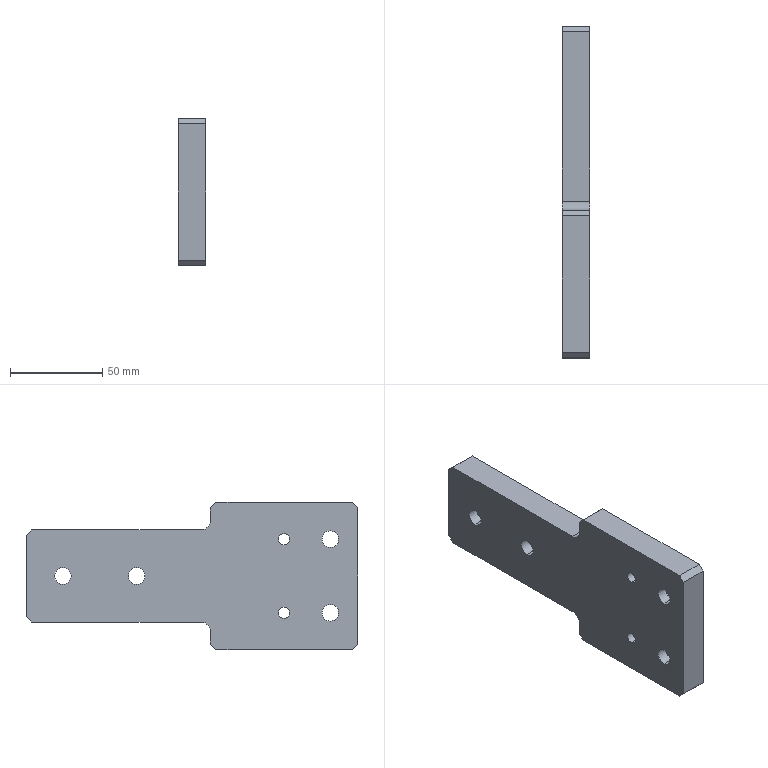Part | SolidWorks | features HoleWzd 4, Chamfer 1, Extrusion 1, Fillet 1 | 1 solid | 54 faces | box 15 x 180 x 80 mm | volume 161661 mm3 | cylinder 26 | plane 20 | cone 8 | commonest cylinder face diameters 9 x8 15 x8 4.2 x4 6 x4 10 x2
STEP:
#1=CARTESIAN_POINT('',(0.,40.,23.));
#2=VERTEX_POINT('',#1);
#3=CARTESIAN_POINT('',(0.,40.,17.));
#4=VERTEX_POINT('',#3);
#5=CARTESIAN_POINT('',(0.,40.,20.));
#6=DIRECTION('',(1.,0.,0.));
#7=DIRECTION('',(0.,0.,-1.));
#8=AXIS2_PLACEMENT_3D('',#5,#6,#7);
#9=CIRCLE('',#8,3.);
#10=EDGE_CURVE('',#2,#4,#9,.T.);
#11=ORIENTED_EDGE('',*,*,#10,.F.);
#12=CARTESIAN_POINT('',(15.,40.,23.));
#13=VERTEX_POINT('',#12);
#14=CARTESIAN_POINT('',(15.,40.,23.));
#15=DIRECTION('',(1.,0.,0.));
#16=VECTOR('',#15,1000.);
#17=LINE('',#14,#16);
#18=EDGE_CURVE('',#2,#13,#17,.T.);
#19=ORIENTED_EDGE('',*,*,#18,.T.);
#20=CARTESIAN_POINT('',(15.,40.,17.));
#21=VERTEX_POINT('',#20);
#22=CARTESIAN_POINT('',(15.,40.,20.));
#23=DIRECTION('',(1.,0.,0.));
#24=DIRECTION('',(0.,0.,-1.));
#25=AXIS2_PLACEMENT_3D('',#22,#23,#24);
#26=CIRCLE('',#25,3.);
#27=EDGE_CURVE('',#13,#21,#26,.T.);
#28=ORIENTED_EDGE('',*,*,#27,.T.);
#29=CARTESIAN_POINT('',(15.,40.,17.));
#30=DIRECTION('',(1.,0.,0.));
#31=VECTOR('',#30,1000.);
#32=LINE('',#29,#31);
#33=EDGE_CURVE('',#4,#21,#32,.T.);
#34=ORIENTED_EDGE('',*,*,#33,.F.);
#35=EDGE_LOOP('',(#11,#19,#28,#34));
#36=FACE_OUTER_BOUND('',#35,.T.);
#37=CARTESIAN_POINT('',(15.,40.,20.));
#38=DIRECTION('',(1.,0.,0.));
#39=DIRECTION('',(0.,0.,-1.));
#40=AXIS2_PLACEMENT_3D('',#37,#38,#39);
#41=CYLINDRICAL_SURFACE('',#40,3.);
#42=ADVANCED_FACE('',(#36),#41,.F.);
#43=CARTESIAN_POINT('',(0.,40.,-17.));
#44=VERTEX_POINT('',#43);
#45=CARTESIAN_POINT('',(0.,40.,-23.));
#46=VERTEX_POINT('',#45);
#47=CARTESIAN_POINT('',(0.,40.,-20.));
#48=DIRECTION('',(1.,0.,0.));
#49=DIRECTION('',(0.,0.,-1.));
#50=AXIS2_PLACEMENT_3D('',#47,#48,#49);
#51=CIRCLE('',#50,3.);
#52=EDGE_CURVE('',#44,#46,#51,.T.);
#53=ORIENTED_EDGE('',*,*,#52,.F.);
#54=CARTESIAN_POINT('',(15.,40.,-17.));
#55=VERTEX_POINT('',#54);
#56=CARTESIAN_POINT('',(15.,40.,-17.));
#57=DIRECTION('',(1.,0.,0.));
#58=VECTOR('',#57,1000.);
#59=LINE('',#56,#58);
#60=EDGE_CURVE('',#44,#55,#59,.T.);
#61=ORIENTED_EDGE('',*,*,#60,.T.);
#62=CARTESIAN_POINT('',(15.,40.,-23.));
#63=VERTEX_POINT('',#62);
#64=CARTESIAN_POINT('',(15.,40.,-20.));
#65=DIRECTION('',(1.,0.,0.));
#66=DIRECTION('',(0.,0.,-1.));
#67=AXIS2_PLACEMENT_3D('',#64,#65,#66);
#68=CIRCLE('',#67,3.);
#69=EDGE_CURVE('',#55,#63,#68,.T.);
#70=ORIENTED_EDGE('',*,*,#69,.T.);
#71=CARTESIAN_POINT('',(15.,40.,-23.));
#72=DIRECTION('',(1.,0.,0.));
#73=VECTOR('',#72,1000.);
#74=LINE('',#71,#73);
#75=EDGE_CURVE('',#46,#63,#74,.T.);
#76=ORIENTED_EDGE('',*,*,#75,.F.);
#77=EDGE_LOOP('',(#53,#61,#70,#76));
#78=FACE_OUTER_BOUND('',#77,.T.);
#79=CARTESIAN_POINT('',(15.,40.,-20.));
#80=DIRECTION('',(1.,0.,0.));
#81=DIRECTION('',(0.,0.,-1.));
#82=AXIS2_PLACEMENT_3D('',#79,#80,#81);
#83=CYLINDRICAL_SURFACE('',#82,3.);
#84=ADVANCED_FACE('',(#78),#83,.F.);
#85=CARTESIAN_POINT('',(6.,15.,27.5));
#86=VERTEX_POINT('',#85);
#87=CARTESIAN_POINT('',(6.,15.,12.5));
#88=VERTEX_POINT('',#87);
#89=CARTESIAN_POINT('',(6.,15.,20.));
#90=DIRECTION('',(1.,0.,0.));
#91=DIRECTION('',(0.,0.,-1.));
#92=AXIS2_PLACEMENT_3D('',#89,#90,#91);
#93=CIRCLE('',#92,7.5);
#94=EDGE_CURVE('',#86,#88,#93,.T.);
#95=ORIENTED_EDGE('',*,*,#94,.F.);
#96=CARTESIAN_POINT('',(15.,15.,27.5));
#97=VERTEX_POINT('',#96);
#98=CARTESIAN_POINT('',(15.,15.,27.5));
#99=DIRECTION('',(1.,0.,0.));
#100=VECTOR('',#99,1000.);
#101=LINE('',#98,#100);
#102=EDGE_CURVE('',#86,#97,#101,.T.);
#103=ORIENTED_EDGE('',*,*,#102,.T.);
#104=CARTESIAN_POINT('',(15.,15.,12.5));
#105=VERTEX_POINT('',#104);
#106=CARTESIAN_POINT('',(15.,15.,20.));
#107=DIRECTION('',(1.,0.,0.));
#108=DIRECTION('',(0.,0.,-1.));
#109=AXIS2_PLACEMENT_3D('',#106,#107,#108);
#110=CIRCLE('',#109,7.5);
#111=EDGE_CURVE('',#97,#105,#110,.T.);
#112=ORIENTED_EDGE('',*,*,#111,.T.);
#113=CARTESIAN_POINT('',(15.,15.,12.5));
#114=DIRECTION('',(1.,0.,0.));
#115=VECTOR('',#114,1000.);
#116=LINE('',#113,#115);
#117=EDGE_CURVE('',#88,#105,#116,.T.);
#118=ORIENTED_EDGE('',*,*,#117,.F.);
#119=EDGE_LOOP('',(#95,#103,#112,#118));
#120=FACE_OUTER_BOUND('',#119,.T.);
#121=CARTESIAN_POINT('',(15.,15.,20.));
#122=DIRECTION('',(1.,0.,0.));
#123=DIRECTION('',(0.,0.,-1.));
#124=AXIS2_PLACEMENT_3D('',#121,#122,#123);
#125=CYLINDRICAL_SURFACE('',#124,7.5);
#126=ADVANCED_FACE('',(#120),#125,.F.);
#127=CARTESIAN_POINT('',(0.,15.,24.5));
#128=VERTEX_POINT('',#127);
#129=CARTESIAN_POINT('',(0.,15.,15.5));
#130=VERTEX_POINT('',#129);
#131=CARTESIAN_POINT('',(0.,15.,20.));
#132=DIRECTION('',(1.,0.,0.));
#133=DIRECTION('',(0.,0.,-1.));
#134=AXIS2_PLACEMENT_3D('',#131,#132,#133);
#135=CIRCLE('',#134,4.5);
#136=EDGE_CURVE('',#128,#130,#135,.T.);
#137=ORIENTED_EDGE('',*,*,#136,.F.);
#138=CARTESIAN_POINT('',(6.,15.,24.5));
#139=VERTEX_POINT('',#138);
#140=CARTESIAN_POINT('',(15.,15.,24.5));
#141=DIRECTION('',(1.,0.,0.));
#142=VECTOR('',#141,1000.);
#143=LINE('',#140,#142);
#144=EDGE_CURVE('',#128,#139,#143,.T.);
#145=ORIENTED_EDGE('',*,*,#144,.T.);
#146=CARTESIAN_POINT('',(6.,15.,15.5));
#147=VERTEX_POINT('',#146);
#148=CARTESIAN_POINT('',(6.,15.,20.));
#149=DIRECTION('',(1.,0.,0.));
#150=DIRECTION('',(0.,0.,-1.));
#151=AXIS2_PLACEMENT_3D('',#148,#149,#150);
#152=CIRCLE('',#151,4.5);
#153=EDGE_CURVE('',#139,#147,#152,.T.);
#154=ORIENTED_EDGE('',*,*,#153,.T.);
#155=CARTESIAN_POINT('',(15.,15.,15.5));
#156=DIRECTION('',(1.,0.,0.));
#157=VECTOR('',#156,1000.);
#158=LINE('',#155,#157);
#159=EDGE_CURVE('',#130,#147,#158,.T.);
#160=ORIENTED_EDGE('',*,*,#159,.F.);
#161=EDGE_LOOP('',(#137,#145,#154,#160));
#162=FACE_OUTER_BOUND('',#161,.T.);
#163=CARTESIAN_POINT('',(15.,15.,20.));
#164=DIRECTION('',(1.,0.,0.));
#165=DIRECTION('',(0.,0.,-1.));
#166=AXIS2_PLACEMENT_3D('',#163,#164,#165);
#167=CYLINDRICAL_SURFACE('',#166,4.5);
#168=ADVANCED_FACE('',(#162),#167,.F.);
#169=CARTESIAN_POINT('',(6.,15.,-12.5));
#170=VERTEX_POINT('',#169);
#171=CARTESIAN_POINT('',(6.,15.,-27.5));
#172=VERTEX_POINT('',#171);
#173=CARTESIAN_POINT('',(6.,15.,-20.));
#174=DIRECTION('',(1.,0.,0.));
#175=DIRECTION('',(0.,0.,-1.));
#176=AXIS2_PLACEMENT_3D('',#173,#174,#175);
#177=CIRCLE('',#176,7.5);
#178=EDGE_CURVE('',#170,#172,#177,.T.);
#179=ORIENTED_EDGE('',*,*,#178,.F.);
#180=CARTESIAN_POINT('',(15.,15.,-12.5));
#181=VERTEX_POINT('',#180);
#182=CARTESIAN_POINT('',(15.,15.,-12.5));
#183=DIRECTION('',(1.,0.,0.));
#184=VECTOR('',#183,1000.);
#185=LINE('',#182,#184);
#186=EDGE_CURVE('',#170,#181,#185,.T.);
#187=ORIENTED_EDGE('',*,*,#186,.T.);
#188=CARTESIAN_POINT('',(15.,15.,-27.5));
#189=VERTEX_POINT('',#188);
#190=CARTESIAN_POINT('',(15.,15.,-20.));
#191=DIRECTION('',(1.,0.,0.));
#192=DIRECTION('',(0.,0.,-1.));
#193=AXIS2_PLACEMENT_3D('',#190,#191,#192);
#194=CIRCLE('',#193,7.5);
#195=EDGE_CURVE('',#181,#189,#194,.T.);
#196=ORIENTED_EDGE('',*,*,#195,.T.);
#197=CARTESIAN_POINT('',(15.,15.,-27.5));
#198=DIRECTION('',(1.,0.,0.));
#199=VECTOR('',#198,1000.);
#200=LINE('',#197,#199);
#201=EDGE_CURVE('',#172,#189,#200,.T.);
#202=ORIENTED_EDGE('',*,*,#201,.F.);
#203=EDGE_LOOP('',(#179,#187,#196,#202));
#204=FACE_OUTER_BOUND('',#203,.T.);
#205=CARTESIAN_POINT('',(15.,15.,-20.));
#206=DIRECTION('',(1.,0.,0.));
#207=DIRECTION('',(0.,0.,-1.));
#208=AXIS2_PLACEMENT_3D('',#205,#206,#207);
#209=CYLINDRICAL_SURFACE('',#208,7.5);
#210=ADVANCED_FACE('',(#204),#209,.F.);
#211=CARTESIAN_POINT('',(0.,15.,-15.5));
#212=VERTEX_POINT('',#211);
#213=CARTESIAN_POINT('',(0.,15.,-24.5));
#214=VERTEX_POINT('',#213);
#215=CARTESIAN_POINT('',(0.,15.,-20.));
#216=DIRECTION('',(1.,0.,0.));
#217=DIRECTION('',(0.,0.,-1.));
#218=AXIS2_PLACEMENT_3D('',#215,#216,#217);
#219=CIRCLE('',#218,4.5);
#220=EDGE_CURVE('',#212,#214,#219,.T.);
#221=ORIENTED_EDGE('',*,*,#220,.F.);
#222=CARTESIAN_POINT('',(6.,15.,-15.5));
#223=VERTEX_POINT('',#222);
#224=CARTESIAN_POINT('',(15.,15.,-15.5));
#225=DIRECTION('',(1.,0.,0.));
#226=VECTOR('',#225,1000.);
#227=LINE('',#224,#226);
#228=EDGE_CURVE('',#212,#223,#227,.T.);
#229=ORIENTED_EDGE('',*,*,#228,.T.);
#230=CARTESIAN_POINT('',(6.,15.,-24.5));
#231=VERTEX_POINT('',#230);
#232=CARTESIAN_POINT('',(6.,15.,-20.));
#233=DIRECTION('',(1.,0.,0.));
#234=DIRECTION('',(0.,0.,-1.));
#235=AXIS2_PLACEMENT_3D('',#232,#233,#234);
#236=CIRCLE('',#235,4.5);
#237=EDGE_CURVE('',#223,#231,#236,.T.);
#238=ORIENTED_EDGE('',*,*,#237,.T.);
#239=CARTESIAN_POINT('',(15.,15.,-24.5));
#240=DIRECTION('',(1.,0.,0.));
#241=VECTOR('',#240,1000.);
#242=LINE('',#239,#241);
#243=EDGE_CURVE('',#214,#231,#242,.T.);
#244=ORIENTED_EDGE('',*,*,#243,.F.);
#245=EDGE_LOOP('',(#221,#229,#238,#244));
#246=FACE_OUTER_BOUND('',#245,.T.);
#247=CARTESIAN_POINT('',(15.,15.,-20.));
#248=DIRECTION('',(1.,0.,0.));
#249=DIRECTION('',(0.,0.,-1.));
#250=AXIS2_PLACEMENT_3D('',#247,#248,#249);
#251=CYLINDRICAL_SURFACE('',#250,4.5);
#252=ADVANCED_FACE('',(#246),#251,.F.);
#253=CARTESIAN_POINT('',(6.,160.,7.5));
#254=VERTEX_POINT('',#253);
#255=CARTESIAN_POINT('',(6.,160.,-7.5));
#256=VERTEX_POINT('',#255);
#257=CARTESIAN_POINT('',(6.,160.,0.));
#258=DIRECTION('',(1.,0.,0.));
#259=DIRECTION('',(0.,0.,-1.));
#260=AXIS2_PLACEMENT_3D('',#257,#258,#259);
#261=CIRCLE('',#260,7.5);
#262=EDGE_CURVE('',#254,#256,#261,.T.);
#263=ORIENTED_EDGE('',*,*,#262,.F.);
#264=CARTESIAN_POINT('',(15.,160.,7.5));
#265=VERTEX_POINT('',#264);
#266=CARTESIAN_POINT('',(15.,160.,7.5));
#267=DIRECTION('',(1.,0.,0.));
#268=VECTOR('',#267,1000.);
#269=LINE('',#266,#268);
#270=EDGE_CURVE('',#254,#265,#269,.T.);
#271=ORIENTED_EDGE('',*,*,#270,.T.);
#272=CARTESIAN_POINT('',(15.,160.,-7.5));
#273=VERTEX_POINT('',#272);
#274=CARTESIAN_POINT('',(15.,160.,0.));
#275=DIRECTION('',(1.,0.,0.));
#276=DIRECTION('',(0.,0.,-1.));
#277=AXIS2_PLACEMENT_3D('',#274,#275,#276);
#278=CIRCLE('',#277,7.5);
#279=EDGE_CURVE('',#265,#273,#278,.T.);
#280=ORIENTED_EDGE('',*,*,#279,.T.);
#281=CARTESIAN_POINT('',(15.,160.,-7.5));
#282=DIRECTION('',(1.,0.,0.));
#283=VECTOR('',#282,1000.);
#284=LINE('',#281,#283);
#285=EDGE_CURVE('',#256,#273,#284,.T.);
#286=ORIENTED_EDGE('',*,*,#285,.F.);
#287=EDGE_LOOP('',(#263,#271,#280,#286));
#288=FACE_OUTER_BOUND('',#287,.T.);
#289=CARTESIAN_POINT('',(15.,160.,0.));
#290=DIRECTION('',(1.,0.,0.));
#291=DIRECTION('',(0.,0.,-1.));
#292=AXIS2_PLACEMENT_3D('',#289,#290,#291);
#293=CYLINDRICAL_SURFACE('',#292,7.5);
#294=ADVANCED_FACE('',(#288),#293,.F.);
#295=CARTESIAN_POINT('',(0.,160.,4.5));
#296=VERTEX_POINT('',#295);
#297=CARTESIAN_POINT('',(0.,160.,-4.5));
#298=VERTEX_POINT('',#297);
#299=CARTESIAN_POINT('',(0.,160.,0.));
#300=DIRECTION('',(1.,0.,0.));
#301=DIRECTION('',(0.,0.,-1.));
#302=AXIS2_PLACEMENT_3D('',#299,#300,#301);
#303=CIRCLE('',#302,4.5);
#304=EDGE_CURVE('',#296,#298,#303,.T.);
#305=ORIENTED_EDGE('',*,*,#304,.F.);
#306=CARTESIAN_POINT('',(6.,160.,4.5));
#307=VERTEX_POINT('',#306);
#308=CARTESIAN_POINT('',(15.,160.,4.5));
#309=DIRECTION('',(1.,0.,0.));
#310=VECTOR('',#309,1000.);
#311=LINE('',#308,#310);
#312=EDGE_CURVE('',#296,#307,#311,.T.);
#313=ORIENTED_EDGE('',*,*,#312,.T.);
#314=CARTESIAN_POINT('',(6.,160.,-4.5));
#315=VERTEX_POINT('',#314);
#316=CARTESIAN_POINT('',(6.,160.,0.));
#317=DIRECTION('',(1.,0.,0.));
#318=DIRECTION('',(0.,0.,-1.));
#319=AXIS2_PLACEMENT_3D('',#316,#317,#318);
#320=CIRCLE('',#319,4.5);
#321=EDGE_CURVE('',#307,#315,#320,.T.);
#322=ORIENTED_EDGE('',*,*,#321,.T.);
#323=CARTESIAN_POINT('',(15.,160.,-4.5));
#324=DIRECTION('',(1.,0.,0.));
#325=VECTOR('',#324,1000.);
#326=LINE('',#323,#325);
#327=EDGE_CURVE('',#298,#315,#326,.T.);
#328=ORIENTED_EDGE('',*,*,#327,.F.);
#329=EDGE_LOOP('',(#305,#313,#322,#328));
#330=FACE_OUTER_BOUND('',#329,.T.);
#331=CARTESIAN_POINT('',(15.,160.,0.));
#332=DIRECTION('',(1.,0.,0.));
#333=DIRECTION('',(0.,0.,-1.));
#334=AXIS2_PLACEMENT_3D('',#331,#332,#333);
#335=CYLINDRICAL_SURFACE('',#334,4.5);
#336=ADVANCED_FACE('',(#330),#335,.F.);
#337=CARTESIAN_POINT('',(6.,120.,7.5));
#338=VERTEX_POINT('',#337);
#339=CARTESIAN_POINT('',(6.,120.,-7.5));
#340=VERTEX_POINT('',#339);
#341=CARTESIAN_POINT('',(6.,120.,0.));
#342=DIRECTION('',(1.,0.,0.));
#343=DIRECTION('',(0.,0.,-1.));
#344=AXIS2_PLACEMENT_3D('',#341,#342,#343);
#345=CIRCLE('',#344,7.5);
#346=EDGE_CURVE('',#338,#340,#345,.T.);
#347=ORIENTED_EDGE('',*,*,#346,.F.);
#348=CARTESIAN_POINT('',(15.,120.,7.5));
#349=VERTEX_POINT('',#348);
#350=CARTESIAN_POINT('',(15.,120.,7.5));
#351=DIRECTION('',(1.,0.,0.));
#352=VECTOR('',#351,1000.);
#353=LINE('',#350,#352);
#354=EDGE_CURVE('',#338,#349,#353,.T.);
#355=ORIENTED_EDGE('',*,*,#354,.T.);
#356=CARTESIAN_POINT('',(15.,120.,-7.5));
#357=VERTEX_POINT('',#356);
#358=CARTESIAN_POINT('',(15.,120.,0.));
#359=DIRECTION('',(1.,0.,0.));
#360=DIRECTION('',(0.,0.,-1.));
#361=AXIS2_PLACEMENT_3D('',#358,#359,#360);
#362=CIRCLE('',#361,7.5);
#363=EDGE_CURVE('',#349,#357,#362,.T.);
#364=ORIENTED_EDGE('',*,*,#363,.T.);
#365=CARTESIAN_POINT('',(15.,120.,-7.5));
#366=DIRECTION('',(1.,0.,0.));
#367=VECTOR('',#366,1000.);
#368=LINE('',#365,#367);
#369=EDGE_CURVE('',#340,#357,#368,.T.);
#370=ORIENTED_EDGE('',*,*,#369,.F.);
#371=EDGE_LOOP('',(#347,#355,#364,#370));
#372=FACE_OUTER_BOUND('',#371,.T.);
#373=CARTESIAN_POINT('',(15.,120.,0.));
#374=DIRECTION('',(1.,0.,0.));
#375=DIRECTION('',(0.,0.,-1.));
#376=AXIS2_PLACEMENT_3D('',#373,#374,#375);
#377=CYLINDRICAL_SURFACE('',#376,7.5);
#378=ADVANCED_FACE('',(#372),#377,.F.);
#379=CARTESIAN_POINT('',(0.,120.,4.5));
#380=VERTEX_POINT('',#379);
#381=CARTESIAN_POINT('',(0.,120.,-4.5));
#382=VERTEX_POINT('',#381);
#383=CARTESIAN_POINT('',(0.,120.,0.));
#384=DIRECTION('',(1.,0.,0.));
#385=DIRECTION('',(0.,0.,-1.));
#386=AXIS2_PLACEMENT_3D('',#383,#384,#385);
#387=CIRCLE('',#386,4.5);
#388=EDGE_CURVE('',#380,#382,#387,.T.);
#389=ORIENTED_EDGE('',*,*,#388,.F.);
#390=CARTESIAN_POINT('',(6.,120.,4.5));
#391=VERTEX_POINT('',#390);
#392=CARTESIAN_POINT('',(15.,120.,4.5));
#393=DIRECTION('',(1.,0.,0.));
#394=VECTOR('',#393,1000.);
#395=LINE('',#392,#394);
#396=EDGE_CURVE('',#380,#391,#395,.T.);
#397=ORIENTED_EDGE('',*,*,#396,.T.);
#398=CARTESIAN_POINT('',(6.,120.,-4.5));
#399=VERTEX_POINT('',#398);
#400=CARTESIAN_POINT('',(6.,120.,0.));
#401=DIRECTION('',(1.,0.,0.));
#402=DIRECTION('',(0.,0.,-1.));
#403=AXIS2_PLACEMENT_3D('',#400,#401,#402);
#404=CIRCLE('',#403,4.5);
#405=EDGE_CURVE('',#391,#399,#404,.T.);
#406=ORIENTED_EDGE('',*,*,#405,.T.);
#407=CARTESIAN_POINT('',(15.,120.,-4.5));
#408=DIRECTION('',(1.,0.,0.));
#409=VECTOR('',#408,1000.);
#410=LINE('',#407,#409);
#411=EDGE_CURVE('',#382,#399,#410,.T.);
#412=ORIENTED_EDGE('',*,*,#411,.F.);
#413=EDGE_LOOP('',(#389,#397,#406,#412));
#414=FACE_OUTER_BOUND('',#413,.T.);
#415=CARTESIAN_POINT('',(15.,120.,0.));
#416=DIRECTION('',(1.,0.,0.));
#417=DIRECTION('',(0.,0.,-1.));
#418=AXIS2_PLACEMENT_3D('',#415,#416,#417);
#419=CYLINDRICAL_SURFACE('',#418,4.5);
#420=ADVANCED_FACE('',(#414),#419,.F.);
#421=CARTESIAN_POINT('',(14.575,29.,-29.4));
#422=VERTEX_POINT('',#421);
#423=CARTESIAN_POINT('',(14.575,29.,-33.6));
#424=VERTEX_POINT('',#423);
#425=CARTESIAN_POINT('',(14.575,29.,-31.5));
#426=DIRECTION('',(1.,0.,0.));
#427=DIRECTION('',(0.,0.,-1.));
#428=AXIS2_PLACEMENT_3D('',#425,#426,#427);
#429=CIRCLE('',#428,2.1);
#430=EDGE_CURVE('',#422,#424,#429,.T.);
#431=ORIENTED_EDGE('',*,*,#430,.F.);
#432=CARTESIAN_POINT('',(15.,29.,-28.975));
#433=VERTEX_POINT('',#432);
#434=CARTESIAN_POINT('',(15.,29.,-28.975));
#435=DIRECTION('',(0.7071,0.,0.7071));
#436=VECTOR('',#435,1000.);
#437=LINE('',#434,#436);
#438=EDGE_CURVE('',#422,#433,#437,.T.);
#439=ORIENTED_EDGE('',*,*,#438,.T.);
#440=CARTESIAN_POINT('',(15.,29.,-34.025));
#441=VERTEX_POINT('',#440);
#442=CARTESIAN_POINT('',(15.,29.,-31.5));
#443=DIRECTION('',(1.,0.,0.));
#444=DIRECTION('',(0.,0.,-1.));
#445=AXIS2_PLACEMENT_3D('',#442,#443,#444);
#446=CIRCLE('',#445,2.525);
#447=EDGE_CURVE('',#433,#441,#446,.T.);
#448=ORIENTED_EDGE('',*,*,#447,.T.);
#449=CARTESIAN_POINT('',(15.,29.,-34.025));
#450=DIRECTION('',(0.7071,0.,-0.7071));
#451=VECTOR('',#450,1000.);
#452=LINE('',#449,#451);
#453=EDGE_CURVE('',#424,#441,#452,.T.);
#454=ORIENTED_EDGE('',*,*,#453,.F.);
#455=EDGE_LOOP('',(#431,#439,#448,#454));
#456=FACE_OUTER_BOUND('',#455,.T.);
#457=CARTESIAN_POINT('',(15.,29.,-31.5));
#458=DIRECTION('',(1.,0.,0.));
#459=DIRECTION('',(0.,0.,-1.));
#460=AXIS2_PLACEMENT_3D('',#457,#458,#459);
#461=CONICAL_SURFACE('',#460,2.525,0.7854);
#462=ADVANCED_FACE('',(#456),#461,.F.);
#463=CARTESIAN_POINT('',(2.6,29.,-29.4));
#464=VERTEX_POINT('',#463);
#465=CARTESIAN_POINT('',(2.6,29.,-33.6));
#466=VERTEX_POINT('',#465);
#467=CARTESIAN_POINT('',(2.6,29.,-31.5));
#468=DIRECTION('',(1.,0.,0.));
#469=DIRECTION('',(0.,0.,-1.));
#470=AXIS2_PLACEMENT_3D('',#467,#468,#469);
#471=CIRCLE('',#470,2.1);
#472=EDGE_CURVE('',#464,#466,#471,.T.);
#473=ORIENTED_EDGE('',*,*,#472,.F.);
#474=CARTESIAN_POINT('',(15.,29.,-29.4));
#475=DIRECTION('',(1.,0.,0.));
#476=VECTOR('',#475,1000.);
#477=LINE('',#474,#476);
#478=EDGE_CURVE('',#464,#422,#477,.T.);
#479=ORIENTED_EDGE('',*,*,#478,.T.);
#480=ORIENTED_EDGE('',*,*,#430,.T.);
#481=CARTESIAN_POINT('',(15.,29.,-33.6));
#482=DIRECTION('',(1.,0.,0.));
#483=VECTOR('',#482,1000.);
#484=LINE('',#481,#483);
#485=EDGE_CURVE('',#466,#424,#484,.T.);
#486=ORIENTED_EDGE('',*,*,#485,.F.);
#487=EDGE_LOOP('',(#473,#479,#480,#486));
#488=FACE_OUTER_BOUND('',#487,.T.);
#489=CARTESIAN_POINT('',(15.,29.,-31.5));
#490=DIRECTION('',(1.,0.,0.));
#491=DIRECTION('',(0.,0.,-1.));
#492=AXIS2_PLACEMENT_3D('',#489,#490,#491);
#493=CYLINDRICAL_SURFACE('',#492,2.1);
#494=ADVANCED_FACE('',(#488),#493,.F.);
#495=CARTESIAN_POINT('',(1.338,29.,-31.5));
#496=VERTEX_POINT('',#495);
#497=CARTESIAN_POINT('',(2.6,29.,-33.6));
#498=DIRECTION('',(0.515,0.,-0.8572));
#499=VECTOR('',#498,1000.);
#500=LINE('',#497,#499);
#501=EDGE_CURVE('',#496,#466,#500,.T.);
#502=ORIENTED_EDGE('',*,*,#501,.F.);
#503=CARTESIAN_POINT('',(2.6,29.,-29.4));
#504=DIRECTION('',(0.515,0.,0.8572));
#505=VECTOR('',#504,1000.);
#506=LINE('',#503,#505);
#507=EDGE_CURVE('',#496,#464,#506,.T.);
#508=ORIENTED_EDGE('',*,*,#507,.T.);
#509=ORIENTED_EDGE('',*,*,#472,.T.);
#510=EDGE_LOOP('',(#502,#508,#509));
#511=FACE_OUTER_BOUND('',#510,.T.);
#512=CARTESIAN_POINT('',(2.6,29.,-31.5));
#513=DIRECTION('',(1.,0.,0.));
#514=DIRECTION('',(0.,0.,-1.));
#515=AXIS2_PLACEMENT_3D('',#512,#513,#514);
#516=CONICAL_SURFACE('',#515,2.1,1.03);
#517=ADVANCED_FACE('',(#511),#516,.F.);
#518=CARTESIAN_POINT('',(14.575,29.,33.6));
#519=VERTEX_POINT('',#518);
#520=CARTESIAN_POINT('',(14.575,29.,29.4));
#521=VERTEX_POINT('',#520);
#522=CARTESIAN_POINT('',(14.575,29.,31.5));
#523=DIRECTION('',(1.,0.,0.));
#524=DIRECTION('',(0.,0.,-1.));
#525=AXIS2_PLACEMENT_3D('',#522,#523,#524);
#526=CIRCLE('',#525,2.1);
#527=EDGE_CURVE('',#519,#521,#526,.T.);
#528=ORIENTED_EDGE('',*,*,#527,.F.);
#529=CARTESIAN_POINT('',(15.,29.,34.025));
#530=VERTEX_POINT('',#529);
#531=CARTESIAN_POINT('',(15.,29.,34.025));
#532=DIRECTION('',(0.7071,0.,0.7071));
#533=VECTOR('',#532,1000.);
#534=LINE('',#531,#533);
#535=EDGE_CURVE('',#519,#530,#534,.T.);
#536=ORIENTED_EDGE('',*,*,#535,.T.);
#537=CARTESIAN_POINT('',(15.,29.,28.975));
#538=VERTEX_POINT('',#537);
#539=CARTESIAN_POINT('',(15.,29.,31.5));
#540=DIRECTION('',(1.,0.,0.));
#541=DIRECTION('',(0.,0.,-1.));
#542=AXIS2_PLACEMENT_3D('',#539,#540,#541);
#543=CIRCLE('',#542,2.525);
#544=EDGE_CURVE('',#530,#538,#543,.T.);
#545=ORIENTED_EDGE('',*,*,#544,.T.);
#546=CARTESIAN_POINT('',(15.,29.,28.975));
#547=DIRECTION('',(0.7071,0.,-0.7071));
#548=VECTOR('',#547,1000.);
#549=LINE('',#546,#548);
#550=EDGE_CURVE('',#521,#538,#549,.T.);
#551=ORIENTED_EDGE('',*,*,#550,.F.);
#552=EDGE_LOOP('',(#528,#536,#545,#551));
#553=FACE_OUTER_BOUND('',#552,.T.);
#554=CARTESIAN_POINT('',(15.,29.,31.5));
#555=DIRECTION('',(1.,0.,0.));
#556=DIRECTION('',(0.,0.,-1.));
#557=AXIS2_PLACEMENT_3D('',#554,#555,#556);
#558=CONICAL_SURFACE('',#557,2.525,0.7854);
#559=ADVANCED_FACE('',(#553),#558,.F.);
#560=CARTESIAN_POINT('',(2.6,29.,33.6));
#561=VERTEX_POINT('',#560);
#562=CARTESIAN_POINT('',(2.6,29.,29.4));
#563=VERTEX_POINT('',#562);
#564=CARTESIAN_POINT('',(2.6,29.,31.5));
#565=DIRECTION('',(1.,0.,0.));
#566=DIRECTION('',(0.,0.,-1.));
#567=AXIS2_PLACEMENT_3D('',#564,#565,#566);
#568=CIRCLE('',#567,2.1);
#569=EDGE_CURVE('',#561,#563,#568,.T.);
#570=ORIENTED_EDGE('',*,*,#569,.F.);
#571=CARTESIAN_POINT('',(15.,29.,33.6));
#572=DIRECTION('',(1.,0.,0.));
#573=VECTOR('',#572,1000.);
#574=LINE('',#571,#573);
#575=EDGE_CURVE('',#561,#519,#574,.T.);
#576=ORIENTED_EDGE('',*,*,#575,.T.);
#577=ORIENTED_EDGE('',*,*,#527,.T.);
#578=CARTESIAN_POINT('',(15.,29.,29.4));
#579=DIRECTION('',(1.,0.,0.));
#580=VECTOR('',#579,1000.);
#581=LINE('',#578,#580);
#582=EDGE_CURVE('',#563,#521,#581,.T.);
#583=ORIENTED_EDGE('',*,*,#582,.F.);
#584=EDGE_LOOP('',(#570,#576,#577,#583));
#585=FACE_OUTER_BOUND('',#584,.T.);
#586=CARTESIAN_POINT('',(15.,29.,31.5));
#587=DIRECTION('',(1.,0.,0.));
#588=DIRECTION('',(0.,0.,-1.));
#589=AXIS2_PLACEMENT_3D('',#586,#587,#588);
#590=CYLINDRICAL_SURFACE('',#589,2.1);
#591=ADVANCED_FACE('',(#585),#590,.F.);
#592=CARTESIAN_POINT('',(1.338,29.,31.5));
#593=VERTEX_POINT('',#592);
#594=CARTESIAN_POINT('',(2.6,29.,29.4));
#595=DIRECTION('',(0.515,0.,-0.8572));
#596=VECTOR('',#595,1000.);
#597=LINE('',#594,#596);
#598=EDGE_CURVE('',#593,#563,#597,.T.);
#599=ORIENTED_EDGE('',*,*,#598,.F.);
#600=CARTESIAN_POINT('',(2.6,29.,33.6));
#601=DIRECTION('',(0.515,0.,0.8572));
#602=VECTOR('',#601,1000.);
#603=LINE('',#600,#602);
#604=EDGE_CURVE('',#593,#561,#603,.T.);
#605=ORIENTED_EDGE('',*,*,#604,.T.);
#606=ORIENTED_EDGE('',*,*,#569,.T.);
#607=EDGE_LOOP('',(#599,#605,#606));
#608=FACE_OUTER_BOUND('',#607,.T.);
#609=CARTESIAN_POINT('',(2.6,29.,31.5));
#610=DIRECTION('',(1.,0.,0.));
#611=DIRECTION('',(0.,0.,-1.));
#612=AXIS2_PLACEMENT_3D('',#609,#610,#611);
#613=CONICAL_SURFACE('',#612,2.1,1.03);
#614=ADVANCED_FACE('',(#608),#613,.F.);
#615=CARTESIAN_POINT('',(0.,80.,30.));
#616=VERTEX_POINT('',#615);
#617=CARTESIAN_POINT('',(0.,80.,37.));
#618=VERTEX_POINT('',#617);
#619=CARTESIAN_POINT('',(0.,80.,40.));
#620=DIRECTION('',(0.,0.,1.));
#621=VECTOR('',#620,1000.);
#622=LINE('',#619,#621);
#623=EDGE_CURVE('',#616,#618,#622,.T.);
#624=ORIENTED_EDGE('',*,*,#623,.T.);
#625=CARTESIAN_POINT('',(15.,80.,37.));
#626=VERTEX_POINT('',#625);
#627=CARTESIAN_POINT('',(15.,80.,37.));
#628=DIRECTION('',(1.,0.,0.));
#629=VECTOR('',#628,1000.);
#630=LINE('',#627,#629);
#631=EDGE_CURVE('',#618,#626,#630,.T.);
#632=ORIENTED_EDGE('',*,*,#631,.T.);
#633=CARTESIAN_POINT('',(15.,80.,30.));
#634=VERTEX_POINT('',#633);
#635=CARTESIAN_POINT('',(15.,80.,40.));
#636=DIRECTION('',(0.,0.,1.));
#637=VECTOR('',#636,1000.);
#638=LINE('',#635,#637);
#639=EDGE_CURVE('',#634,#626,#638,.T.);
#640=ORIENTED_EDGE('',*,*,#639,.F.);
#641=CARTESIAN_POINT('',(0.,80.,30.));
#642=DIRECTION('',(-1.,0.,0.));
#643=VECTOR('',#642,1000.);
#644=LINE('',#641,#643);
#645=EDGE_CURVE('',#634,#616,#644,.T.);
#646=ORIENTED_EDGE('',*,*,#645,.T.);
#647=EDGE_LOOP('',(#624,#632,#640,#646));
#648=FACE_OUTER_BOUND('',#647,.T.);
#649=CARTESIAN_POINT('',(15.,80.,40.));
#650=DIRECTION('',(0.,-1.,0.));
#651=DIRECTION('',(0.,0.,-1.));
#652=AXIS2_PLACEMENT_3D('',#649,#650,#651);
#653=PLANE('',#652);
#654=ADVANCED_FACE('',(#648),#653,.F.);
#655=CARTESIAN_POINT('',(0.,77.,40.));
#656=VERTEX_POINT('',#655);
#657=CARTESIAN_POINT('',(0.,3.,40.));
#658=VERTEX_POINT('',#657);
#659=CARTESIAN_POINT('',(0.,0.,40.));
#660=DIRECTION('',(0.,-1.,0.));
#661=VECTOR('',#660,1000.);
#662=LINE('',#659,#661);
#663=EDGE_CURVE('',#656,#658,#662,.T.);
#664=ORIENTED_EDGE('',*,*,#663,.T.);
#665=CARTESIAN_POINT('',(15.,3.,40.));
#666=VERTEX_POINT('',#665);
#667=CARTESIAN_POINT('',(15.,3.,40.));
#668=DIRECTION('',(1.,0.,0.));
#669=VECTOR('',#668,1000.);
#670=LINE('',#667,#669);
#671=EDGE_CURVE('',#658,#666,#670,.T.);
#672=ORIENTED_EDGE('',*,*,#671,.T.);
#673=CARTESIAN_POINT('',(15.,77.,40.));
#674=VERTEX_POINT('',#673);
#675=CARTESIAN_POINT('',(15.,0.,40.));
#676=DIRECTION('',(0.,-1.,0.));
#677=VECTOR('',#676,1000.);
#678=LINE('',#675,#677);
#679=EDGE_CURVE('',#674,#666,#678,.T.);
#680=ORIENTED_EDGE('',*,*,#679,.F.);
#681=CARTESIAN_POINT('',(15.,77.,40.));
#682=DIRECTION('',(-1.,0.,0.));
#683=VECTOR('',#682,1000.);
#684=LINE('',#681,#683);
#685=EDGE_CURVE('',#674,#656,#684,.T.);
#686=ORIENTED_EDGE('',*,*,#685,.T.);
#687=EDGE_LOOP('',(#664,#672,#680,#686));
#688=FACE_OUTER_BOUND('',#687,.T.);
#689=CARTESIAN_POINT('',(15.,0.,40.));
#690=DIRECTION('',(0.,0.,-1.));
#691=DIRECTION('',(-1.,0.,0.));
#692=AXIS2_PLACEMENT_3D('',#689,#690,#691);
#693=PLANE('',#692);
#694=ADVANCED_FACE('',(#688),#693,.F.);
#695=CARTESIAN_POINT('',(0.,0.,37.));
#696=VERTEX_POINT('',#695);
#697=CARTESIAN_POINT('',(0.,0.,-37.));
#698=VERTEX_POINT('',#697);
#699=CARTESIAN_POINT('',(0.,0.,-40.));
#700=DIRECTION('',(0.,0.,-1.));
#701=VECTOR('',#700,1000.);
#702=LINE('',#699,#701);
#703=EDGE_CURVE('',#696,#698,#702,.T.);
#704=ORIENTED_EDGE('',*,*,#703,.T.);
#705=CARTESIAN_POINT('',(15.,0.,-37.));
#706=VERTEX_POINT('',#705);
#707=CARTESIAN_POINT('',(15.,0.,-37.));
#708=DIRECTION('',(1.,0.,0.));
#709=VECTOR('',#708,1000.);
#710=LINE('',#707,#709);
#711=EDGE_CURVE('',#698,#706,#710,.T.);
#712=ORIENTED_EDGE('',*,*,#711,.T.);
#713=CARTESIAN_POINT('',(15.,0.,37.));
#714=VERTEX_POINT('',#713);
#715=CARTESIAN_POINT('',(15.,0.,-40.));
#716=DIRECTION('',(0.,0.,-1.));
#717=VECTOR('',#716,1000.);
#718=LINE('',#715,#717);
#719=EDGE_CURVE('',#714,#706,#718,.T.);
#720=ORIENTED_EDGE('',*,*,#719,.F.);
#721=CARTESIAN_POINT('',(15.,0.,37.));
#722=DIRECTION('',(-1.,0.,0.));
#723=VECTOR('',#722,1000.);
#724=LINE('',#721,#723);
#725=EDGE_CURVE('',#714,#696,#724,.T.);
#726=ORIENTED_EDGE('',*,*,#725,.T.);
#727=EDGE_LOOP('',(#704,#712,#720,#726));
#728=FACE_OUTER_BOUND('',#727,.T.);
#729=CARTESIAN_POINT('',(15.,0.,-40.));
#730=DIRECTION('',(0.,1.,0.));
#731=DIRECTION('',(0.,0.,1.));
#732=AXIS2_PLACEMENT_3D('',#729,#730,#731);
#733=PLANE('',#732);
#734=ADVANCED_FACE('',(#728),#733,.F.);
#735=CARTESIAN_POINT('',(0.,3.,-40.));
#736=VERTEX_POINT('',#735);
#737=CARTESIAN_POINT('',(0.,77.,-40.));
#738=VERTEX_POINT('',#737);
#739=CARTESIAN_POINT('',(0.,0.,-40.));
#740=DIRECTION('',(0.,1.,0.));
#741=VECTOR('',#740,1000.);
#742=LINE('',#739,#741);
#743=EDGE_CURVE('',#736,#738,#742,.T.);
#744=ORIENTED_EDGE('',*,*,#743,.T.);
#745=CARTESIAN_POINT('',(15.,77.,-40.));
#746=VERTEX_POINT('',#745);
#747=CARTESIAN_POINT('',(15.,77.,-40.));
#748=DIRECTION('',(1.,0.,0.));
#749=VECTOR('',#748,1000.);
#750=LINE('',#747,#749);
#751=EDGE_CURVE('',#738,#746,#750,.T.);
#752=ORIENTED_EDGE('',*,*,#751,.T.);
#753=CARTESIAN_POINT('',(15.,3.,-40.));
#754=VERTEX_POINT('',#753);
#755=CARTESIAN_POINT('',(15.,0.,-40.));
#756=DIRECTION('',(0.,1.,0.));
#757=VECTOR('',#756,1000.);
#758=LINE('',#755,#757);
#759=EDGE_CURVE('',#754,#746,#758,.T.);
#760=ORIENTED_EDGE('',*,*,#759,.F.);
#761=CARTESIAN_POINT('',(15.,3.,-40.));
#762=DIRECTION('',(-1.,0.,0.));
#763=VECTOR('',#762,1000.);
#764=LINE('',#761,#763);
#765=EDGE_CURVE('',#754,#736,#764,.T.);
#766=ORIENTED_EDGE('',*,*,#765,.T.);
#767=EDGE_LOOP('',(#744,#752,#760,#766));
#768=FACE_OUTER_BOUND('',#767,.T.);
#769=CARTESIAN_POINT('',(15.,0.,-40.));
#770=DIRECTION('',(0.,0.,1.));
#771=DIRECTION('',(1.,0.,0.));
#772=AXIS2_PLACEMENT_3D('',#769,#770,#771);
#773=PLANE('',#772);
#774=ADVANCED_FACE('',(#768),#773,.F.);
#775=CARTESIAN_POINT('',(15.,80.,-37.));
#776=VERTEX_POINT('',#775);
#777=CARTESIAN_POINT('',(15.,80.,-30.));
#778=VERTEX_POINT('',#777);
#779=CARTESIAN_POINT('',(15.,80.,-40.));
#780=DIRECTION('',(0.,0.,1.));
#781=VECTOR('',#780,1000.);
#782=LINE('',#779,#781);
#783=EDGE_CURVE('',#776,#778,#782,.T.);
#784=ORIENTED_EDGE('',*,*,#783,.F.);
#785=CARTESIAN_POINT('',(0.,80.,-37.));
#786=VERTEX_POINT('',#785);
#787=CARTESIAN_POINT('',(15.,80.,-37.));
#788=DIRECTION('',(-1.,0.,0.));
#789=VECTOR('',#788,1000.);
#790=LINE('',#787,#789);
#791=EDGE_CURVE('',#776,#786,#790,.T.);
#792=ORIENTED_EDGE('',*,*,#791,.T.);
#793=CARTESIAN_POINT('',(0.,80.,-30.));
#794=VERTEX_POINT('',#793);
#795=CARTESIAN_POINT('',(0.,80.,-40.));
#796=DIRECTION('',(0.,0.,1.));
#797=VECTOR('',#796,1000.);
#798=LINE('',#795,#797);
#799=EDGE_CURVE('',#786,#794,#798,.T.);
#800=ORIENTED_EDGE('',*,*,#799,.T.);
#801=CARTESIAN_POINT('',(15.,80.,-30.));
#802=DIRECTION('',(1.,0.,0.));
#803=VECTOR('',#802,1000.);
#804=LINE('',#801,#803);
#805=EDGE_CURVE('',#794,#778,#804,.T.);
#806=ORIENTED_EDGE('',*,*,#805,.T.);
#807=EDGE_LOOP('',(#784,#792,#800,#806));
#808=FACE_OUTER_BOUND('',#807,.T.);
#809=CARTESIAN_POINT('',(15.,80.,-40.));
#810=DIRECTION('',(0.,-1.,0.));
#811=DIRECTION('',(0.,0.,-1.));
#812=AXIS2_PLACEMENT_3D('',#809,#810,#811);
#813=PLANE('',#812);
#814=ADVANCED_FACE('',(#808),#813,.F.);
#815=CARTESIAN_POINT('',(0.,85.,-25.));
#816=VERTEX_POINT('',#815);
#817=CARTESIAN_POINT('',(0.,177.,-25.));
#818=VERTEX_POINT('',#817);
#819=CARTESIAN_POINT('',(0.,80.,-25.));
#820=DIRECTION('',(0.,1.,0.));
#821=VECTOR('',#820,1000.);
#822=LINE('',#819,#821);
#823=EDGE_CURVE('',#816,#818,#822,.T.);
#824=ORIENTED_EDGE('',*,*,#823,.T.);
#825=CARTESIAN_POINT('',(15.,177.,-25.));
#826=VERTEX_POINT('',#825);
#827=CARTESIAN_POINT('',(15.,177.,-25.));
#828=DIRECTION('',(1.,0.,0.));
#829=VECTOR('',#828,1000.);
#830=LINE('',#827,#829);
#831=EDGE_CURVE('',#818,#826,#830,.T.);
#832=ORIENTED_EDGE('',*,*,#831,.T.);
#833=CARTESIAN_POINT('',(15.,85.,-25.));
#834=VERTEX_POINT('',#833);
#835=CARTESIAN_POINT('',(15.,80.,-25.));
#836=DIRECTION('',(0.,1.,0.));
#837=VECTOR('',#836,1000.);
#838=LINE('',#835,#837);
#839=EDGE_CURVE('',#834,#826,#838,.T.);
#840=ORIENTED_EDGE('',*,*,#839,.F.);
#841=CARTESIAN_POINT('',(0.,85.,-25.));
#842=DIRECTION('',(-1.,0.,0.));
#843=VECTOR('',#842,1000.);
#844=LINE('',#841,#843);
#845=EDGE_CURVE('',#834,#816,#844,.T.);
#846=ORIENTED_EDGE('',*,*,#845,.T.);
#847=EDGE_LOOP('',(#824,#832,#840,#846));
#848=FACE_OUTER_BOUND('',#847,.T.);
#849=CARTESIAN_POINT('',(15.,80.,-25.));
#850=DIRECTION('',(0.,0.,1.));
#851=DIRECTION('',(1.,0.,0.));
#852=AXIS2_PLACEMENT_3D('',#849,#850,#851);
#853=PLANE('',#852);
#854=ADVANCED_FACE('',(#848),#853,.F.);
#855=CARTESIAN_POINT('',(15.,180.,-22.));
#856=VERTEX_POINT('',#855);
#857=CARTESIAN_POINT('',(15.,180.,22.));
#858=VERTEX_POINT('',#857);
#859=CARTESIAN_POINT('',(15.,180.,25.));
#860=DIRECTION('',(0.,0.,1.));
#861=VECTOR('',#860,1000.);
#862=LINE('',#859,#861);
#863=EDGE_CURVE('',#856,#858,#862,.T.);
#864=ORIENTED_EDGE('',*,*,#863,.F.);
#865=CARTESIAN_POINT('',(0.,180.,-22.));
#866=VERTEX_POINT('',#865);
#867=CARTESIAN_POINT('',(15.,180.,-22.));
#868=DIRECTION('',(-1.,0.,0.));
#869=VECTOR('',#868,1000.);
#870=LINE('',#867,#869);
#871=EDGE_CURVE('',#856,#866,#870,.T.);
#872=ORIENTED_EDGE('',*,*,#871,.T.);
#873=CARTESIAN_POINT('',(0.,180.,22.));
#874=VERTEX_POINT('',#873);
#875=CARTESIAN_POINT('',(0.,180.,25.));
#876=DIRECTION('',(0.,0.,1.));
#877=VECTOR('',#876,1000.);
#878=LINE('',#875,#877);
#879=EDGE_CURVE('',#866,#874,#878,.T.);
#880=ORIENTED_EDGE('',*,*,#879,.T.);
#881=CARTESIAN_POINT('',(15.,180.,22.));
#882=DIRECTION('',(1.,0.,0.));
#883=VECTOR('',#882,1000.);
#884=LINE('',#881,#883);
#885=EDGE_CURVE('',#874,#858,#884,.T.);
#886=ORIENTED_EDGE('',*,*,#885,.T.);
#887=EDGE_LOOP('',(#864,#872,#880,#886));
#888=FACE_OUTER_BOUND('',#887,.T.);
#889=CARTESIAN_POINT('',(15.,180.,25.));
#890=DIRECTION('',(0.,-1.,0.));
#891=DIRECTION('',(0.,0.,-1.));
#892=AXIS2_PLACEMENT_3D('',#889,#890,#891);
#893=PLANE('',#892);
#894=ADVANCED_FACE('',(#888),#893,.F.);
#895=CARTESIAN_POINT('',(15.,177.,25.));
#896=VERTEX_POINT('',#895);
#897=CARTESIAN_POINT('',(15.,85.,25.));
#898=VERTEX_POINT('',#897);
#899=CARTESIAN_POINT('',(15.,80.,25.));
#900=DIRECTION('',(0.,-1.,0.));
#901=VECTOR('',#900,1000.);
#902=LINE('',#899,#901);
#903=EDGE_CURVE('',#896,#898,#902,.T.);
#904=ORIENTED_EDGE('',*,*,#903,.F.);
#905=CARTESIAN_POINT('',(0.,177.,25.));
#906=VERTEX_POINT('',#905);
#907=CARTESIAN_POINT('',(15.,177.,25.));
#908=DIRECTION('',(-1.,0.,0.));
#909=VECTOR('',#908,1000.);
#910=LINE('',#907,#909);
#911=EDGE_CURVE('',#896,#906,#910,.T.);
#912=ORIENTED_EDGE('',*,*,#911,.T.);
#913=CARTESIAN_POINT('',(0.,85.,25.));
#914=VERTEX_POINT('',#913);
#915=CARTESIAN_POINT('',(0.,80.,25.));
#916=DIRECTION('',(0.,-1.,0.));
#917=VECTOR('',#916,1000.);
#918=LINE('',#915,#917);
#919=EDGE_CURVE('',#906,#914,#918,.T.);
#920=ORIENTED_EDGE('',*,*,#919,.T.);
#921=CARTESIAN_POINT('',(15.,85.,25.));
#922=DIRECTION('',(1.,0.,0.));
#923=VECTOR('',#922,1000.);
#924=LINE('',#921,#923);
#925=EDGE_CURVE('',#914,#898,#924,.T.);
#926=ORIENTED_EDGE('',*,*,#925,.T.);
#927=EDGE_LOOP('',(#904,#912,#920,#926));
#928=FACE_OUTER_BOUND('',#927,.T.);
#929=CARTESIAN_POINT('',(15.,80.,25.));
#930=DIRECTION('',(0.,0.,-1.));
#931=DIRECTION('',(-1.,0.,0.));
#932=AXIS2_PLACEMENT_3D('',#929,#930,#931);
#933=PLANE('',#932);
#934=ADVANCED_FACE('',(#928),#933,.F.);
#935=CARTESIAN_POINT('',(15.,40.,20.));
#936=DIRECTION('',(1.,0.,0.));
#937=DIRECTION('',(0.,0.,-1.));
#938=AXIS2_PLACEMENT_3D('',#935,#936,#937);
#939=CIRCLE('',#938,3.);
#940=EDGE_CURVE('',#21,#13,#939,.T.);
#941=ORIENTED_EDGE('',*,*,#940,.F.);
#942=ORIENTED_EDGE('',*,*,#27,.F.);
#943=EDGE_LOOP('',(#941,#942));
#944=FACE_BOUND('',#943,.T.);
#945=CARTESIAN_POINT('',(15.,40.,-20.));
#946=DIRECTION('',(1.,0.,0.));
#947=DIRECTION('',(0.,0.,-1.));
#948=AXIS2_PLACEMENT_3D('',#945,#946,#947);
#949=CIRCLE('',#948,3.);
#950=EDGE_CURVE('',#63,#55,#949,.T.);
#951=ORIENTED_EDGE('',*,*,#950,.F.);
#952=ORIENTED_EDGE('',*,*,#69,.F.);
#953=EDGE_LOOP('',(#951,#952));
#954=FACE_BOUND('',#953,.T.);
#955=CARTESIAN_POINT('',(15.,15.,20.));
#956=DIRECTION('',(1.,0.,0.));
#957=DIRECTION('',(0.,0.,-1.));
#958=AXIS2_PLACEMENT_3D('',#955,#956,#957);
#959=CIRCLE('',#958,7.5);
#960=EDGE_CURVE('',#105,#97,#959,.T.);
#961=ORIENTED_EDGE('',*,*,#960,.F.);
#962=ORIENTED_EDGE('',*,*,#111,.F.);
#963=EDGE_LOOP('',(#961,#962));
#964=FACE_BOUND('',#963,.T.);
#965=CARTESIAN_POINT('',(15.,15.,-20.));
#966=DIRECTION('',(1.,0.,0.));
#967=DIRECTION('',(0.,0.,-1.));
#968=AXIS2_PLACEMENT_3D('',#965,#966,#967);
#969=CIRCLE('',#968,7.5);
#970=EDGE_CURVE('',#189,#181,#969,.T.);
#971=ORIENTED_EDGE('',*,*,#970,.F.);
#972=ORIENTED_EDGE('',*,*,#195,.F.);
#973=EDGE_LOOP('',(#971,#972));
#974=FACE_BOUND('',#973,.T.);
#975=CARTESIAN_POINT('',(15.,160.,0.));
#976=DIRECTION('',(1.,0.,0.));
#977=DIRECTION('',(0.,0.,-1.));
#978=AXIS2_PLACEMENT_3D('',#975,#976,#977);
#979=CIRCLE('',#978,7.5);
#980=EDGE_CURVE('',#273,#265,#979,.T.);
#981=ORIENTED_EDGE('',*,*,#980,.F.);
#982=ORIENTED_EDGE('',*,*,#279,.F.);
#983=EDGE_LOOP('',(#981,#982));
#984=FACE_BOUND('',#983,.T.);
#985=CARTESIAN_POINT('',(15.,120.,0.));
#986=DIRECTION('',(1.,0.,0.));
#987=DIRECTION('',(0.,0.,-1.));
#988=AXIS2_PLACEMENT_3D('',#985,#986,#987);
#989=CIRCLE('',#988,7.5);
#990=EDGE_CURVE('',#357,#349,#989,.T.);
#991=ORIENTED_EDGE('',*,*,#990,.F.);
#992=ORIENTED_EDGE('',*,*,#363,.F.);
#993=EDGE_LOOP('',(#991,#992));
#994=FACE_BOUND('',#993,.T.);
#995=CARTESIAN_POINT('',(15.,29.,-31.5));
#996=DIRECTION('',(1.,0.,0.));
#997=DIRECTION('',(0.,0.,-1.));
#998=AXIS2_PLACEMENT_3D('',#995,#996,#997);
#999=CIRCLE('',#998,2.525);
#1000=EDGE_CURVE('',#441,#433,#999,.T.);
#1001=ORIENTED_EDGE('',*,*,#1000,.F.);
#1002=ORIENTED_EDGE('',*,*,#447,.F.);
#1003=EDGE_LOOP('',(#1001,#1002));
#1004=FACE_BOUND('',#1003,.T.);
#1005=CARTESIAN_POINT('',(15.,29.,31.5));
#1006=DIRECTION('',(1.,0.,0.));
#1007=DIRECTION('',(0.,0.,-1.));
#1008=AXIS2_PLACEMENT_3D('',#1005,#1006,#1007);
#1009=CIRCLE('',#1008,2.525);
#1010=EDGE_CURVE('',#538,#530,#1009,.T.);
#1011=ORIENTED_EDGE('',*,*,#1010,.F.);
#1012=ORIENTED_EDGE('',*,*,#544,.F.);
#1013=EDGE_LOOP('',(#1011,#1012));
#1014=FACE_BOUND('',#1013,.T.);
#1015=ORIENTED_EDGE('',*,*,#839,.T.);
#1016=CARTESIAN_POINT('',(15.,101.,-101.));
#1017=DIRECTION('',(0.,0.7071,0.7071));
#1018=VECTOR('',#1017,1000.);
#1019=LINE('',#1016,#1018);
#1020=EDGE_CURVE('',#826,#856,#1019,.T.);
#1021=ORIENTED_EDGE('',*,*,#1020,.T.);
#1022=ORIENTED_EDGE('',*,*,#863,.T.);
#1023=CARTESIAN_POINT('',(15.,101.,101.));
#1024=DIRECTION('',(0.,-0.7071,0.7071));
#1025=VECTOR('',#1024,1000.);
#1026=LINE('',#1023,#1025);
#1027=EDGE_CURVE('',#858,#896,#1026,.T.);
#1028=ORIENTED_EDGE('',*,*,#1027,.T.);
#1029=ORIENTED_EDGE('',*,*,#903,.T.);
#1030=CARTESIAN_POINT('',(15.,85.,30.));
#1031=DIRECTION('',(-1.,0.,0.));
#1032=DIRECTION('',(0.,0.,-1.));
#1033=AXIS2_PLACEMENT_3D('',#1030,#1031,#1032);
#1034=CIRCLE('',#1033,5.);
#1035=EDGE_CURVE('',#898,#634,#1034,.T.);
#1036=ORIENTED_EDGE('',*,*,#1035,.T.);
#1037=ORIENTED_EDGE('',*,*,#639,.T.);
#1038=CARTESIAN_POINT('',(15.,58.5,58.5));
#1039=DIRECTION('',(0.,-0.7071,0.7071));
#1040=VECTOR('',#1039,1000.);
#1041=LINE('',#1038,#1040);
#1042=EDGE_CURVE('',#626,#674,#1041,.T.);
#1043=ORIENTED_EDGE('',*,*,#1042,.T.);
#1044=ORIENTED_EDGE('',*,*,#679,.T.);
#1045=CARTESIAN_POINT('',(15.,-18.5,18.5));
#1046=DIRECTION('',(0.,-0.7071,-0.7071));
#1047=VECTOR('',#1046,1000.);
#1048=LINE('',#1045,#1047);
#1049=EDGE_CURVE('',#666,#714,#1048,.T.);
#1050=ORIENTED_EDGE('',*,*,#1049,.T.);
#1051=ORIENTED_EDGE('',*,*,#719,.T.);
#1052=CARTESIAN_POINT('',(15.,-18.5,-18.5));
#1053=DIRECTION('',(0.,0.7071,-0.7071));
#1054=VECTOR('',#1053,1000.);
#1055=LINE('',#1052,#1054);
#1056=EDGE_CURVE('',#706,#754,#1055,.T.);
#1057=ORIENTED_EDGE('',*,*,#1056,.T.);
#1058=ORIENTED_EDGE('',*,*,#759,.T.);
#1059=CARTESIAN_POINT('',(15.,58.5,-58.5));
#1060=DIRECTION('',(0.,0.7071,0.7071));
#1061=VECTOR('',#1060,1000.);
#1062=LINE('',#1059,#1061);
#1063=EDGE_CURVE('',#746,#776,#1062,.T.);
#1064=ORIENTED_EDGE('',*,*,#1063,.T.);
#1065=ORIENTED_EDGE('',*,*,#783,.T.);
#1066=CARTESIAN_POINT('',(15.,85.,-30.));
#1067=DIRECTION('',(-1.,0.,0.));
#1068=DIRECTION('',(0.,0.,-1.));
#1069=AXIS2_PLACEMENT_3D('',#1066,#1067,#1068);
#1070=CIRCLE('',#1069,5.);
#1071=EDGE_CURVE('',#778,#834,#1070,.T.);
#1072=ORIENTED_EDGE('',*,*,#1071,.T.);
#1073=EDGE_LOOP('',(#1015,#1021,#1022,#1028,#1029,#1036,#1037,#1043,#1044,#1050,#1051,#1057,#1058,#1064,#1065,#1072));
#1074=FACE_OUTER_BOUND('',#1073,.T.);
#1075=CARTESIAN_POINT('',(15.,0.,0.));
#1076=DIRECTION('',(1.,0.,0.));
#1077=DIRECTION('',(0.,0.,-1.));
#1078=AXIS2_PLACEMENT_3D('',#1075,#1076,#1077);
#1079=PLANE('',#1078);
#1080=ADVANCED_FACE('',(#944,#954,#964,#974,#984,#994,#1004,#1014,#1074),#1079,.T.);
#1081=CARTESIAN_POINT('',(0.,40.,20.));
#1082=DIRECTION('',(1.,0.,0.));
#1083=DIRECTION('',(0.,0.,-1.));
#1084=AXIS2_PLACEMENT_3D('',#1081,#1082,#1083);
#1085=CIRCLE('',#1084,3.);
#1086=EDGE_CURVE('',#4,#2,#1085,.T.);
#1087=ORIENTED_EDGE('',*,*,#1086,.T.);
#1088=ORIENTED_EDGE('',*,*,#10,.T.);
#1089=EDGE_LOOP('',(#1087,#1088));
#1090=FACE_BOUND('',#1089,.T.);
#1091=CARTESIAN_POINT('',(0.,40.,-20.));
#1092=DIRECTION('',(1.,0.,0.));
#1093=DIRECTION('',(0.,0.,-1.));
#1094=AXIS2_PLACEMENT_3D('',#1091,#1092,#1093);
#1095=CIRCLE('',#1094,3.);
#1096=EDGE_CURVE('',#46,#44,#1095,.T.);
#1097=ORIENTED_EDGE('',*,*,#1096,.T.);
#1098=ORIENTED_EDGE('',*,*,#52,.T.);
#1099=EDGE_LOOP('',(#1097,#1098));
#1100=FACE_BOUND('',#1099,.T.);
#1101=CARTESIAN_POINT('',(0.,15.,20.));
#1102=DIRECTION('',(1.,0.,0.));
#1103=DIRECTION('',(0.,0.,-1.));
#1104=AXIS2_PLACEMENT_3D('',#1101,#1102,#1103);
#1105=CIRCLE('',#1104,4.5);
#1106=EDGE_CURVE('',#130,#128,#1105,.T.);
#1107=ORIENTED_EDGE('',*,*,#1106,.T.);
#1108=ORIENTED_EDGE('',*,*,#136,.T.);
#1109=EDGE_LOOP('',(#1107,#1108));
#1110=FACE_BOUND('',#1109,.T.);
#1111=CARTESIAN_POINT('',(0.,15.,-20.));
#1112=DIRECTION('',(1.,0.,0.));
#1113=DIRECTION('',(0.,0.,-1.));
#1114=AXIS2_PLACEMENT_3D('',#1111,#1112,#1113);
#1115=CIRCLE('',#1114,4.5);
#1116=EDGE_CURVE('',#214,#212,#1115,.T.);
#1117=ORIENTED_EDGE('',*,*,#1116,.T.);
#1118=ORIENTED_EDGE('',*,*,#220,.T.);
#1119=EDGE_LOOP('',(#1117,#1118));
#1120=FACE_BOUND('',#1119,.T.);
#1121=CARTESIAN_POINT('',(0.,160.,0.));
#1122=DIRECTION('',(1.,0.,0.));
#1123=DIRECTION('',(0.,0.,-1.));
#1124=AXIS2_PLACEMENT_3D('',#1121,#1122,#1123);
#1125=CIRCLE('',#1124,4.5);
#1126=EDGE_CURVE('',#298,#296,#1125,.T.);
#1127=ORIENTED_EDGE('',*,*,#1126,.T.);
#1128=ORIENTED_EDGE('',*,*,#304,.T.);
#1129=EDGE_LOOP('',(#1127,#1128));
#1130=FACE_BOUND('',#1129,.T.);
#1131=CARTESIAN_POINT('',(0.,120.,0.));
#1132=DIRECTION('',(1.,0.,0.));
#1133=DIRECTION('',(0.,0.,-1.));
#1134=AXIS2_PLACEMENT_3D('',#1131,#1132,#1133);
#1135=CIRCLE('',#1134,4.5);
#1136=EDGE_CURVE('',#382,#380,#1135,.T.);
#1137=ORIENTED_EDGE('',*,*,#1136,.T.);
#1138=ORIENTED_EDGE('',*,*,#388,.T.);
#1139=EDGE_LOOP('',(#1137,#1138));
#1140=FACE_BOUND('',#1139,.T.);
#1141=ORIENTED_EDGE('',*,*,#879,.F.);
#1142=CARTESIAN_POINT('',(0.,180.,-22.));
#1143=DIRECTION('',(0.,-0.7071,-0.7071));
#1144=VECTOR('',#1143,1000.);
#1145=LINE('',#1142,#1144);
#1146=EDGE_CURVE('',#866,#818,#1145,.T.);
#1147=ORIENTED_EDGE('',*,*,#1146,.T.);
#1148=ORIENTED_EDGE('',*,*,#823,.F.);
#1149=CARTESIAN_POINT('',(0.,85.,-30.));
#1150=DIRECTION('',(1.,0.,0.));
#1151=DIRECTION('',(0.,0.,-1.));
#1152=AXIS2_PLACEMENT_3D('',#1149,#1150,#1151);
#1153=CIRCLE('',#1152,5.);
#1154=EDGE_CURVE('',#816,#794,#1153,.T.);
#1155=ORIENTED_EDGE('',*,*,#1154,.T.);
#1156=ORIENTED_EDGE('',*,*,#799,.F.);
#1157=CARTESIAN_POINT('',(0.,80.,-37.));
#1158=DIRECTION('',(0.,-0.7071,-0.7071));
#1159=VECTOR('',#1158,1000.);
#1160=LINE('',#1157,#1159);
#1161=EDGE_CURVE('',#786,#738,#1160,.T.);
#1162=ORIENTED_EDGE('',*,*,#1161,.T.);
#1163=ORIENTED_EDGE('',*,*,#743,.F.);
#1164=CARTESIAN_POINT('',(0.,3.,-40.));
#1165=DIRECTION('',(0.,-0.7071,0.7071));
#1166=VECTOR('',#1165,1000.);
#1167=LINE('',#1164,#1166);
#1168=EDGE_CURVE('',#736,#698,#1167,.T.);
#1169=ORIENTED_EDGE('',*,*,#1168,.T.);
#1170=ORIENTED_EDGE('',*,*,#703,.F.);
#1171=CARTESIAN_POINT('',(0.,0.,37.));
#1172=DIRECTION('',(0.,0.7071,0.7071));
#1173=VECTOR('',#1172,1000.);
#1174=LINE('',#1171,#1173);
#1175=EDGE_CURVE('',#696,#658,#1174,.T.);
#1176=ORIENTED_EDGE('',*,*,#1175,.T.);
#1177=ORIENTED_EDGE('',*,*,#663,.F.);
#1178=CARTESIAN_POINT('',(0.,77.,40.));
#1179=DIRECTION('',(0.,0.7071,-0.7071));
#1180=VECTOR('',#1179,1000.);
#1181=LINE('',#1178,#1180);
#1182=EDGE_CURVE('',#656,#618,#1181,.T.);
#1183=ORIENTED_EDGE('',*,*,#1182,.T.);
#1184=ORIENTED_EDGE('',*,*,#623,.F.);
#1185=CARTESIAN_POINT('',(0.,85.,30.));
#1186=DIRECTION('',(1.,0.,0.));
#1187=DIRECTION('',(0.,0.,-1.));
#1188=AXIS2_PLACEMENT_3D('',#1185,#1186,#1187);
#1189=CIRCLE('',#1188,5.);
#1190=EDGE_CURVE('',#616,#914,#1189,.T.);
#1191=ORIENTED_EDGE('',*,*,#1190,.T.);
#1192=ORIENTED_EDGE('',*,*,#919,.F.);
#1193=CARTESIAN_POINT('',(0.,177.,25.));
#1194=DIRECTION('',(0.,0.7071,-0.7071));
#1195=VECTOR('',#1194,1000.);
#1196=LINE('',#1193,#1195);
#1197=EDGE_CURVE('',#906,#874,#1196,.T.);
#1198=ORIENTED_EDGE('',*,*,#1197,.T.);
#1199=EDGE_LOOP('',(#1141,#1147,#1148,#1155,#1156,#1162,#1163,#1169,#1170,#1176,#1177,#1183,#1184,#1191,#1192,#1198));
#1200=FACE_OUTER_BOUND('',#1199,.T.);
#1201=CARTESIAN_POINT('',(0.,0.,0.));
#1202=DIRECTION('',(1.,0.,0.));
#1203=DIRECTION('',(0.,0.,-1.));
#1204=AXIS2_PLACEMENT_3D('',#1201,#1202,#1203);
#1205=PLANE('',#1204);
#1206=ADVANCED_FACE('',(#1090,#1100,#1110,#1120,#1130,#1140,#1200),#1205,.F.);
#1207=ORIENTED_EDGE('',*,*,#604,.F.);
#1208=ORIENTED_EDGE('',*,*,#598,.T.);
#1209=CARTESIAN_POINT('',(2.6,29.,31.5));
#1210=DIRECTION('',(1.,0.,0.));
#1211=DIRECTION('',(0.,0.,-1.));
#1212=AXIS2_PLACEMENT_3D('',#1209,#1210,#1211);
#1213=CIRCLE('',#1212,2.1);
#1214=EDGE_CURVE('',#563,#561,#1213,.T.);
#1215=ORIENTED_EDGE('',*,*,#1214,.T.);
#1216=EDGE_LOOP('',(#1207,#1208,#1215));
#1217=FACE_OUTER_BOUND('',#1216,.T.);
#1218=CARTESIAN_POINT('',(2.6,29.,31.5));
#1219=DIRECTION('',(1.,0.,0.));
#1220=DIRECTION('',(0.,0.,-1.));
#1221=AXIS2_PLACEMENT_3D('',#1218,#1219,#1220);
#1222=CONICAL_SURFACE('',#1221,2.1,1.03);
#1223=ADVANCED_FACE('',(#1217),#1222,.F.);
#1224=ORIENTED_EDGE('',*,*,#575,.F.);
#1225=ORIENTED_EDGE('',*,*,#1214,.F.);
#1226=ORIENTED_EDGE('',*,*,#582,.T.);
#1227=CARTESIAN_POINT('',(14.575,29.,31.5));
#1228=DIRECTION('',(1.,0.,0.));
#1229=DIRECTION('',(0.,0.,-1.));
#1230=AXIS2_PLACEMENT_3D('',#1227,#1228,#1229);
#1231=CIRCLE('',#1230,2.1);
#1232=EDGE_CURVE('',#521,#519,#1231,.T.);
#1233=ORIENTED_EDGE('',*,*,#1232,.T.);
#1234=EDGE_LOOP('',(#1224,#1225,#1226,#1233));
#1235=FACE_OUTER_BOUND('',#1234,.T.);
#1236=CARTESIAN_POINT('',(15.,29.,31.5));
#1237=DIRECTION('',(1.,0.,0.));
#1238=DIRECTION('',(0.,0.,-1.));
#1239=AXIS2_PLACEMENT_3D('',#1236,#1237,#1238);
#1240=CYLINDRICAL_SURFACE('',#1239,2.1);
#1241=ADVANCED_FACE('',(#1235),#1240,.F.);
#1242=ORIENTED_EDGE('',*,*,#535,.F.);
#1243=ORIENTED_EDGE('',*,*,#1232,.F.);
#1244=ORIENTED_EDGE('',*,*,#550,.T.);
#1245=ORIENTED_EDGE('',*,*,#1010,.T.);
#1246=EDGE_LOOP('',(#1242,#1243,#1244,#1245));
#1247=FACE_OUTER_BOUND('',#1246,.T.);
#1248=CARTESIAN_POINT('',(15.,29.,31.5));
#1249=DIRECTION('',(1.,0.,0.));
#1250=DIRECTION('',(0.,0.,-1.));
#1251=AXIS2_PLACEMENT_3D('',#1248,#1249,#1250);
#1252=CONICAL_SURFACE('',#1251,2.525,0.7854);
#1253=ADVANCED_FACE('',(#1247),#1252,.F.);
#1254=ORIENTED_EDGE('',*,*,#507,.F.);
#1255=ORIENTED_EDGE('',*,*,#501,.T.);
#1256=CARTESIAN_POINT('',(2.6,29.,-31.5));
#1257=DIRECTION('',(1.,0.,0.));
#1258=DIRECTION('',(0.,0.,-1.));
#1259=AXIS2_PLACEMENT_3D('',#1256,#1257,#1258);
#1260=CIRCLE('',#1259,2.1);
#1261=EDGE_CURVE('',#466,#464,#1260,.T.);
#1262=ORIENTED_EDGE('',*,*,#1261,.T.);
#1263=EDGE_LOOP('',(#1254,#1255,#1262));
#1264=FACE_OUTER_BOUND('',#1263,.T.);
#1265=CARTESIAN_POINT('',(2.6,29.,-31.5));
#1266=DIRECTION('',(1.,0.,0.));
#1267=DIRECTION('',(0.,0.,-1.));
#1268=AXIS2_PLACEMENT_3D('',#1265,#1266,#1267);
#1269=CONICAL_SURFACE('',#1268,2.1,1.03);
#1270=ADVANCED_FACE('',(#1264),#1269,.F.);
#1271=ORIENTED_EDGE('',*,*,#478,.F.);
#1272=ORIENTED_EDGE('',*,*,#1261,.F.);
#1273=ORIENTED_EDGE('',*,*,#485,.T.);
#1274=CARTESIAN_POINT('',(14.575,29.,-31.5));
#1275=DIRECTION('',(1.,0.,0.));
#1276=DIRECTION('',(0.,0.,-1.));
#1277=AXIS2_PLACEMENT_3D('',#1274,#1275,#1276);
#1278=CIRCLE('',#1277,2.1);
#1279=EDGE_CURVE('',#424,#422,#1278,.T.);
#1280=ORIENTED_EDGE('',*,*,#1279,.T.);
#1281=EDGE_LOOP('',(#1271,#1272,#1273,#1280));
#1282=FACE_OUTER_BOUND('',#1281,.T.);
#1283=CARTESIAN_POINT('',(15.,29.,-31.5));
#1284=DIRECTION('',(1.,0.,0.));
#1285=DIRECTION('',(0.,0.,-1.));
#1286=AXIS2_PLACEMENT_3D('',#1283,#1284,#1285);
#1287=CYLINDRICAL_SURFACE('',#1286,2.1);
#1288=ADVANCED_FACE('',(#1282),#1287,.F.);
#1289=ORIENTED_EDGE('',*,*,#438,.F.);
#1290=ORIENTED_EDGE('',*,*,#1279,.F.);
#1291=ORIENTED_EDGE('',*,*,#453,.T.);
#1292=ORIENTED_EDGE('',*,*,#1000,.T.);
#1293=EDGE_LOOP('',(#1289,#1290,#1291,#1292));
#1294=FACE_OUTER_BOUND('',#1293,.T.);
#1295=CARTESIAN_POINT('',(15.,29.,-31.5));
#1296=DIRECTION('',(1.,0.,0.));
#1297=DIRECTION('',(0.,0.,-1.));
#1298=AXIS2_PLACEMENT_3D('',#1295,#1296,#1297);
#1299=CONICAL_SURFACE('',#1298,2.525,0.7854);
#1300=ADVANCED_FACE('',(#1294),#1299,.F.);
#1301=ORIENTED_EDGE('',*,*,#396,.F.);
#1302=ORIENTED_EDGE('',*,*,#1136,.F.);
#1303=ORIENTED_EDGE('',*,*,#411,.T.);
#1304=CARTESIAN_POINT('',(6.,120.,0.));
#1305=DIRECTION('',(1.,0.,0.));
#1306=DIRECTION('',(0.,0.,-1.));
#1307=AXIS2_PLACEMENT_3D('',#1304,#1305,#1306);
#1308=CIRCLE('',#1307,4.5);
#1309=EDGE_CURVE('',#399,#391,#1308,.T.);
#1310=ORIENTED_EDGE('',*,*,#1309,.T.);
#1311=EDGE_LOOP('',(#1301,#1302,#1303,#1310));
#1312=FACE_OUTER_BOUND('',#1311,.T.);
#1313=CARTESIAN_POINT('',(15.,120.,0.));
#1314=DIRECTION('',(1.,0.,0.));
#1315=DIRECTION('',(0.,0.,-1.));
#1316=AXIS2_PLACEMENT_3D('',#1313,#1314,#1315);
#1317=CYLINDRICAL_SURFACE('',#1316,4.5);
#1318=ADVANCED_FACE('',(#1312),#1317,.F.);
#1319=ORIENTED_EDGE('',*,*,#1309,.F.);
#1320=ORIENTED_EDGE('',*,*,#405,.F.);
#1321=EDGE_LOOP('',(#1319,#1320));
#1322=FACE_BOUND('',#1321,.T.);
#1323=CARTESIAN_POINT('',(6.,120.,0.));
#1324=DIRECTION('',(1.,0.,0.));
#1325=DIRECTION('',(0.,0.,-1.));
#1326=AXIS2_PLACEMENT_3D('',#1323,#1324,#1325);
#1327=CIRCLE('',#1326,7.5);
#1328=EDGE_CURVE('',#340,#338,#1327,.T.);
#1329=ORIENTED_EDGE('',*,*,#1328,.T.);
#1330=ORIENTED_EDGE('',*,*,#346,.T.);
#1331=EDGE_LOOP('',(#1329,#1330));
#1332=FACE_OUTER_BOUND('',#1331,.T.);
#1333=CARTESIAN_POINT('',(6.,124.5,0.));
#1334=DIRECTION('',(-1.,0.,0.));
#1335=DIRECTION('',(0.,0.,1.));
#1336=AXIS2_PLACEMENT_3D('',#1333,#1334,#1335);
#1337=PLANE('',#1336);
#1338=ADVANCED_FACE('',(#1322,#1332),#1337,.F.);
#1339=ORIENTED_EDGE('',*,*,#354,.F.);
#1340=ORIENTED_EDGE('',*,*,#1328,.F.);
#1341=ORIENTED_EDGE('',*,*,#369,.T.);
#1342=ORIENTED_EDGE('',*,*,#990,.T.);
#1343=EDGE_LOOP('',(#1339,#1340,#1341,#1342));
#1344=FACE_OUTER_BOUND('',#1343,.T.);
#1345=CARTESIAN_POINT('',(15.,120.,0.));
#1346=DIRECTION('',(1.,0.,0.));
#1347=DIRECTION('',(0.,0.,-1.));
#1348=AXIS2_PLACEMENT_3D('',#1345,#1346,#1347);
#1349=CYLINDRICAL_SURFACE('',#1348,7.5);
#1350=ADVANCED_FACE('',(#1344),#1349,.F.);
#1351=ORIENTED_EDGE('',*,*,#312,.F.);
#1352=ORIENTED_EDGE('',*,*,#1126,.F.);
#1353=ORIENTED_EDGE('',*,*,#327,.T.);
#1354=CARTESIAN_POINT('',(6.,160.,0.));
#1355=DIRECTION('',(1.,0.,0.));
#1356=DIRECTION('',(0.,0.,-1.));
#1357=AXIS2_PLACEMENT_3D('',#1354,#1355,#1356);
#1358=CIRCLE('',#1357,4.5);
#1359=EDGE_CURVE('',#315,#307,#1358,.T.);
#1360=ORIENTED_EDGE('',*,*,#1359,.T.);
#1361=EDGE_LOOP('',(#1351,#1352,#1353,#1360));
#1362=FACE_OUTER_BOUND('',#1361,.T.);
#1363=CARTESIAN_POINT('',(15.,160.,0.));
#1364=DIRECTION('',(1.,0.,0.));
#1365=DIRECTION('',(0.,0.,-1.));
#1366=AXIS2_PLACEMENT_3D('',#1363,#1364,#1365);
#1367=CYLINDRICAL_SURFACE('',#1366,4.5);
#1368=ADVANCED_FACE('',(#1362),#1367,.F.);
#1369=ORIENTED_EDGE('',*,*,#1359,.F.);
#1370=ORIENTED_EDGE('',*,*,#321,.F.);
#1371=EDGE_LOOP('',(#1369,#1370));
#1372=FACE_BOUND('',#1371,.T.);
#1373=CARTESIAN_POINT('',(6.,160.,0.));
#1374=DIRECTION('',(1.,0.,0.));
#1375=DIRECTION('',(0.,0.,-1.));
#1376=AXIS2_PLACEMENT_3D('',#1373,#1374,#1375);
#1377=CIRCLE('',#1376,7.5);
#1378=EDGE_CURVE('',#256,#254,#1377,.T.);
#1379=ORIENTED_EDGE('',*,*,#1378,.T.);
#1380=ORIENTED_EDGE('',*,*,#262,.T.);
#1381=EDGE_LOOP('',(#1379,#1380));
#1382=FACE_OUTER_BOUND('',#1381,.T.);
#1383=CARTESIAN_POINT('',(6.,164.5,0.));
#1384=DIRECTION('',(-1.,0.,0.));
#1385=DIRECTION('',(0.,0.,1.));
#1386=AXIS2_PLACEMENT_3D('',#1383,#1384,#1385);
#1387=PLANE('',#1386);
#1388=ADVANCED_FACE('',(#1372,#1382),#1387,.F.);
#1389=ORIENTED_EDGE('',*,*,#270,.F.);
#1390=ORIENTED_EDGE('',*,*,#1378,.F.);
#1391=ORIENTED_EDGE('',*,*,#285,.T.);
#1392=ORIENTED_EDGE('',*,*,#980,.T.);
#1393=EDGE_LOOP('',(#1389,#1390,#1391,#1392));
#1394=FACE_OUTER_BOUND('',#1393,.T.);
#1395=CARTESIAN_POINT('',(15.,160.,0.));
#1396=DIRECTION('',(1.,0.,0.));
#1397=DIRECTION('',(0.,0.,-1.));
#1398=AXIS2_PLACEMENT_3D('',#1395,#1396,#1397);
#1399=CYLINDRICAL_SURFACE('',#1398,7.5);
#1400=ADVANCED_FACE('',(#1394),#1399,.F.);
#1401=ORIENTED_EDGE('',*,*,#228,.F.);
#1402=ORIENTED_EDGE('',*,*,#1116,.F.);
#1403=ORIENTED_EDGE('',*,*,#243,.T.);
#1404=CARTESIAN_POINT('',(6.,15.,-20.));
#1405=DIRECTION('',(1.,0.,0.));
#1406=DIRECTION('',(0.,0.,-1.));
#1407=AXIS2_PLACEMENT_3D('',#1404,#1405,#1406);
#1408=CIRCLE('',#1407,4.5);
#1409=EDGE_CURVE('',#231,#223,#1408,.T.);
#1410=ORIENTED_EDGE('',*,*,#1409,.T.);
#1411=EDGE_LOOP('',(#1401,#1402,#1403,#1410));
#1412=FACE_OUTER_BOUND('',#1411,.T.);
#1413=CARTESIAN_POINT('',(15.,15.,-20.));
#1414=DIRECTION('',(1.,0.,0.));
#1415=DIRECTION('',(0.,0.,-1.));
#1416=AXIS2_PLACEMENT_3D('',#1413,#1414,#1415);
#1417=CYLINDRICAL_SURFACE('',#1416,4.5);
#1418=ADVANCED_FACE('',(#1412),#1417,.F.);
#1419=ORIENTED_EDGE('',*,*,#1409,.F.);
#1420=ORIENTED_EDGE('',*,*,#237,.F.);
#1421=EDGE_LOOP('',(#1419,#1420));
#1422=FACE_BOUND('',#1421,.T.);
#1423=CARTESIAN_POINT('',(6.,15.,-20.));
#1424=DIRECTION('',(1.,0.,0.));
#1425=DIRECTION('',(0.,0.,-1.));
#1426=AXIS2_PLACEMENT_3D('',#1423,#1424,#1425);
#1427=CIRCLE('',#1426,7.5);
#1428=EDGE_CURVE('',#172,#170,#1427,.T.);
#1429=ORIENTED_EDGE('',*,*,#1428,.T.);
#1430=ORIENTED_EDGE('',*,*,#178,.T.);
#1431=EDGE_LOOP('',(#1429,#1430));
#1432=FACE_OUTER_BOUND('',#1431,.T.);
#1433=CARTESIAN_POINT('',(6.,19.5,-20.));
#1434=DIRECTION('',(-1.,0.,0.));
#1435=DIRECTION('',(0.,0.,1.));
#1436=AXIS2_PLACEMENT_3D('',#1433,#1434,#1435);
#1437=PLANE('',#1436);
#1438=ADVANCED_FACE('',(#1422,#1432),#1437,.F.);
#1439=ORIENTED_EDGE('',*,*,#186,.F.);
#1440=ORIENTED_EDGE('',*,*,#1428,.F.);
#1441=ORIENTED_EDGE('',*,*,#201,.T.);
#1442=ORIENTED_EDGE('',*,*,#970,.T.);
#1443=EDGE_LOOP('',(#1439,#1440,#1441,#1442));
#1444=FACE_OUTER_BOUND('',#1443,.T.);
#1445=CARTESIAN_POINT('',(15.,15.,-20.));
#1446=DIRECTION('',(1.,0.,0.));
#1447=DIRECTION('',(0.,0.,-1.));
#1448=AXIS2_PLACEMENT_3D('',#1445,#1446,#1447);
#1449=CYLINDRICAL_SURFACE('',#1448,7.5);
#1450=ADVANCED_FACE('',(#1444),#1449,.F.);
#1451=ORIENTED_EDGE('',*,*,#144,.F.);
#1452=ORIENTED_EDGE('',*,*,#1106,.F.);
#1453=ORIENTED_EDGE('',*,*,#159,.T.);
#1454=CARTESIAN_POINT('',(6.,15.,20.));
#1455=DIRECTION('',(1.,0.,0.));
#1456=DIRECTION('',(0.,0.,-1.));
#1457=AXIS2_PLACEMENT_3D('',#1454,#1455,#1456);
#1458=CIRCLE('',#1457,4.5);
#1459=EDGE_CURVE('',#147,#139,#1458,.T.);
#1460=ORIENTED_EDGE('',*,*,#1459,.T.);
#1461=EDGE_LOOP('',(#1451,#1452,#1453,#1460));
#1462=FACE_OUTER_BOUND('',#1461,.T.);
#1463=CARTESIAN_POINT('',(15.,15.,20.));
#1464=DIRECTION('',(1.,0.,0.));
#1465=DIRECTION('',(0.,0.,-1.));
#1466=AXIS2_PLACEMENT_3D('',#1463,#1464,#1465);
#1467=CYLINDRICAL_SURFACE('',#1466,4.5);
#1468=ADVANCED_FACE('',(#1462),#1467,.F.);
#1469=ORIENTED_EDGE('',*,*,#1459,.F.);
#1470=ORIENTED_EDGE('',*,*,#153,.F.);
#1471=EDGE_LOOP('',(#1469,#1470));
#1472=FACE_BOUND('',#1471,.T.);
#1473=CARTESIAN_POINT('',(6.,15.,20.));
#1474=DIRECTION('',(1.,0.,0.));
#1475=DIRECTION('',(0.,0.,-1.));
#1476=AXIS2_PLACEMENT_3D('',#1473,#1474,#1475);
#1477=CIRCLE('',#1476,7.5);
#1478=EDGE_CURVE('',#88,#86,#1477,.T.);
#1479=ORIENTED_EDGE('',*,*,#1478,.T.);
#1480=ORIENTED_EDGE('',*,*,#94,.T.);
#1481=EDGE_LOOP('',(#1479,#1480));
#1482=FACE_OUTER_BOUND('',#1481,.T.);
#1483=CARTESIAN_POINT('',(6.,19.5,20.));
#1484=DIRECTION('',(-1.,0.,0.));
#1485=DIRECTION('',(0.,0.,1.));
#1486=AXIS2_PLACEMENT_3D('',#1483,#1484,#1485);
#1487=PLANE('',#1486);
#1488=ADVANCED_FACE('',(#1472,#1482),#1487,.F.);
#1489=ORIENTED_EDGE('',*,*,#102,.F.);
#1490=ORIENTED_EDGE('',*,*,#1478,.F.);
#1491=ORIENTED_EDGE('',*,*,#117,.T.);
#1492=ORIENTED_EDGE('',*,*,#960,.T.);
#1493=EDGE_LOOP('',(#1489,#1490,#1491,#1492));
#1494=FACE_OUTER_BOUND('',#1493,.T.);
#1495=CARTESIAN_POINT('',(15.,15.,20.));
#1496=DIRECTION('',(1.,0.,0.));
#1497=DIRECTION('',(0.,0.,-1.));
#1498=AXIS2_PLACEMENT_3D('',#1495,#1496,#1497);
#1499=CYLINDRICAL_SURFACE('',#1498,7.5);
#1500=ADVANCED_FACE('',(#1494),#1499,.F.);
#1501=ORIENTED_EDGE('',*,*,#60,.F.);
#1502=ORIENTED_EDGE('',*,*,#1096,.F.);
#1503=ORIENTED_EDGE('',*,*,#75,.T.);
#1504=ORIENTED_EDGE('',*,*,#950,.T.);
#1505=EDGE_LOOP('',(#1501,#1502,#1503,#1504));
#1506=FACE_OUTER_BOUND('',#1505,.T.);
#1507=CARTESIAN_POINT('',(15.,40.,-20.));
#1508=DIRECTION('',(1.,0.,0.));
#1509=DIRECTION('',(0.,0.,-1.));
#1510=AXIS2_PLACEMENT_3D('',#1507,#1508,#1509);
#1511=CYLINDRICAL_SURFACE('',#1510,3.);
#1512=ADVANCED_FACE('',(#1506),#1511,.F.);
#1513=ORIENTED_EDGE('',*,*,#18,.F.);
#1514=ORIENTED_EDGE('',*,*,#1086,.F.);
#1515=ORIENTED_EDGE('',*,*,#33,.T.);
#1516=ORIENTED_EDGE('',*,*,#940,.T.);
#1517=EDGE_LOOP('',(#1513,#1514,#1515,#1516));
#1518=FACE_OUTER_BOUND('',#1517,.T.);
#1519=CARTESIAN_POINT('',(15.,40.,20.));
#1520=DIRECTION('',(1.,0.,0.));
#1521=DIRECTION('',(0.,0.,-1.));
#1522=AXIS2_PLACEMENT_3D('',#1519,#1520,#1521);
#1523=CYLINDRICAL_SURFACE('',#1522,3.);
#1524=ADVANCED_FACE('',(#1518),#1523,.F.);
#1525=ORIENTED_EDGE('',*,*,#1071,.F.);
#1526=ORIENTED_EDGE('',*,*,#805,.F.);
#1527=ORIENTED_EDGE('',*,*,#1154,.F.);
#1528=ORIENTED_EDGE('',*,*,#845,.F.);
#1529=EDGE_LOOP('',(#1525,#1526,#1527,#1528));
#1530=FACE_OUTER_BOUND('',#1529,.T.);
#1531=CARTESIAN_POINT('',(15.,85.,-30.));
#1532=DIRECTION('',(1.,0.,0.));
#1533=DIRECTION('',(0.,0.,-1.));
#1534=AXIS2_PLACEMENT_3D('',#1531,#1532,#1533);
#1535=CYLINDRICAL_SURFACE('',#1534,5.);
#1536=ADVANCED_FACE('',(#1530),#1535,.F.);
#1537=ORIENTED_EDGE('',*,*,#1035,.F.);
#1538=ORIENTED_EDGE('',*,*,#925,.F.);
#1539=ORIENTED_EDGE('',*,*,#1190,.F.);
#1540=ORIENTED_EDGE('',*,*,#645,.F.);
#1541=EDGE_LOOP('',(#1537,#1538,#1539,#1540));
#1542=FACE_OUTER_BOUND('',#1541,.T.);
#1543=CARTESIAN_POINT('',(15.,85.,30.));
#1544=DIRECTION('',(1.,0.,0.));
#1545=DIRECTION('',(0.,0.,-1.));
#1546=AXIS2_PLACEMENT_3D('',#1543,#1544,#1545);
#1547=CYLINDRICAL_SURFACE('',#1546,5.);
#1548=ADVANCED_FACE('',(#1542),#1547,.F.);
#1549=ORIENTED_EDGE('',*,*,#1020,.F.);
#1550=ORIENTED_EDGE('',*,*,#831,.F.);
#1551=ORIENTED_EDGE('',*,*,#1146,.F.);
#1552=ORIENTED_EDGE('',*,*,#871,.F.);
#1553=EDGE_LOOP('',(#1549,#1550,#1551,#1552));
#1554=FACE_OUTER_BOUND('',#1553,.T.);
#1555=CARTESIAN_POINT('',(15.,180.,-22.));
#1556=DIRECTION('',(0.,-0.7071,0.7071));
#1557=DIRECTION('',(-1.,0.,0.));
#1558=AXIS2_PLACEMENT_3D('',#1555,#1556,#1557);
#1559=PLANE('',#1558);
#1560=ADVANCED_FACE('',(#1554),#1559,.F.);
#1561=ORIENTED_EDGE('',*,*,#1063,.F.);
#1562=ORIENTED_EDGE('',*,*,#751,.F.);
#1563=ORIENTED_EDGE('',*,*,#1161,.F.);
#1564=ORIENTED_EDGE('',*,*,#791,.F.);
#1565=EDGE_LOOP('',(#1561,#1562,#1563,#1564));
#1566=FACE_OUTER_BOUND('',#1565,.T.);
#1567=CARTESIAN_POINT('',(15.,80.,-37.));
#1568=DIRECTION('',(0.,-0.7071,0.7071));
#1569=DIRECTION('',(-1.,0.,0.));
#1570=AXIS2_PLACEMENT_3D('',#1567,#1568,#1569);
#1571=PLANE('',#1570);
#1572=ADVANCED_FACE('',(#1566),#1571,.F.);
#1573=ORIENTED_EDGE('',*,*,#1056,.F.);
#1574=ORIENTED_EDGE('',*,*,#711,.F.);
#1575=ORIENTED_EDGE('',*,*,#1168,.F.);
#1576=ORIENTED_EDGE('',*,*,#765,.F.);
#1577=EDGE_LOOP('',(#1573,#1574,#1575,#1576));
#1578=FACE_OUTER_BOUND('',#1577,.T.);
#1579=CARTESIAN_POINT('',(15.,3.,-40.));
#1580=DIRECTION('',(0.,0.7071,0.7071));
#1581=DIRECTION('',(-1.,0.,0.));
#1582=AXIS2_PLACEMENT_3D('',#1579,#1580,#1581);
#1583=PLANE('',#1582);
#1584=ADVANCED_FACE('',(#1578),#1583,.F.);
#1585=ORIENTED_EDGE('',*,*,#1049,.F.);
#1586=ORIENTED_EDGE('',*,*,#671,.F.);
#1587=ORIENTED_EDGE('',*,*,#1175,.F.);
#1588=ORIENTED_EDGE('',*,*,#725,.F.);
#1589=EDGE_LOOP('',(#1585,#1586,#1587,#1588));
#1590=FACE_OUTER_BOUND('',#1589,.T.);
#1591=CARTESIAN_POINT('',(15.,0.,37.));
#1592=DIRECTION('',(0.,0.7071,-0.7071));
#1593=DIRECTION('',(-1.,0.,0.));
#1594=AXIS2_PLACEMENT_3D('',#1591,#1592,#1593);
#1595=PLANE('',#1594);
#1596=ADVANCED_FACE('',(#1590),#1595,.F.);
#1597=ORIENTED_EDGE('',*,*,#1042,.F.);
#1598=ORIENTED_EDGE('',*,*,#631,.F.);
#1599=ORIENTED_EDGE('',*,*,#1182,.F.);
#1600=ORIENTED_EDGE('',*,*,#685,.F.);
#1601=EDGE_LOOP('',(#1597,#1598,#1599,#1600));
#1602=FACE_OUTER_BOUND('',#1601,.T.);
#1603=CARTESIAN_POINT('',(15.,77.,40.));
#1604=DIRECTION('',(0.,-0.7071,-0.7071));
#1605=DIRECTION('',(-1.,0.,0.));
#1606=AXIS2_PLACEMENT_3D('',#1603,#1604,#1605);
#1607=PLANE('',#1606);
#1608=ADVANCED_FACE('',(#1602),#1607,.F.);
#1609=ORIENTED_EDGE('',*,*,#1027,.F.);
#1610=ORIENTED_EDGE('',*,*,#885,.F.);
#1611=ORIENTED_EDGE('',*,*,#1197,.F.);
#1612=ORIENTED_EDGE('',*,*,#911,.F.);
#1613=EDGE_LOOP('',(#1609,#1610,#1611,#1612));
#1614=FACE_OUTER_BOUND('',#1613,.T.);
#1615=CARTESIAN_POINT('',(15.,177.,25.));
#1616=DIRECTION('',(0.,-0.7071,-0.7071));
#1617=DIRECTION('',(-1.,0.,0.));
#1618=AXIS2_PLACEMENT_3D('',#1615,#1616,#1617);
#1619=PLANE('',#1618);
#1620=ADVANCED_FACE('',(#1614),#1619,.F.);
#1621=CLOSED_SHELL('',(#42,#84,#126,#168,#210,#252,#294,#336,#378,#420,#462,#494,#517,#559,#591,#614,#654,#694,#734,#774,#814,#854,#894,#934,#1080,#1206,#1223,#1241,#1253,#1270,#1288,#1300,#1318,#1338,#1350,#1368,#1388,#1400,#1418,#1438,#1450,#1468,#1488,#1500,#1512,#1524,#1536,#1548,#1560,#1572,#1584,#1596,#1608,#1620));
#1622=MANIFOLD_SOLID_BREP('',#1621);
#1623=CARTESIAN_POINT('',(0.,0.,0.));
#1624=DIRECTION('',(0.,0.,1.));
#1625=DIRECTION('',(1.,0.,0.));
#1626=AXIS2_PLACEMENT_3D('',#1623,#1624,#1625);
#1627=(LENGTH_UNIT()NAMED_UNIT(*)SI_UNIT(.MILLI.,.METRE.));
#1628=UNCERTAINTY_MEASURE_WITH_UNIT(LENGTH_MEASURE(0.00001),#1627,'','');
#1629=(NAMED_UNIT(*)PLANE_ANGLE_UNIT()SI_UNIT($,.RADIAN.));
#1630=(NAMED_UNIT(*)SI_UNIT($,.STERADIAN.)SOLID_ANGLE_UNIT());
#1631=(GEOMETRIC_REPRESENTATION_CONTEXT(3)GLOBAL_UNCERTAINTY_ASSIGNED_CONTEXT((#1628))GLOBAL_UNIT_ASSIGNED_CONTEXT((#1627,#1629,#1630))REPRESENTATION_CONTEXT('',''));
#1632=ADVANCED_BREP_SHAPE_REPRESENTATION('',(#1622,#1626),#1631);